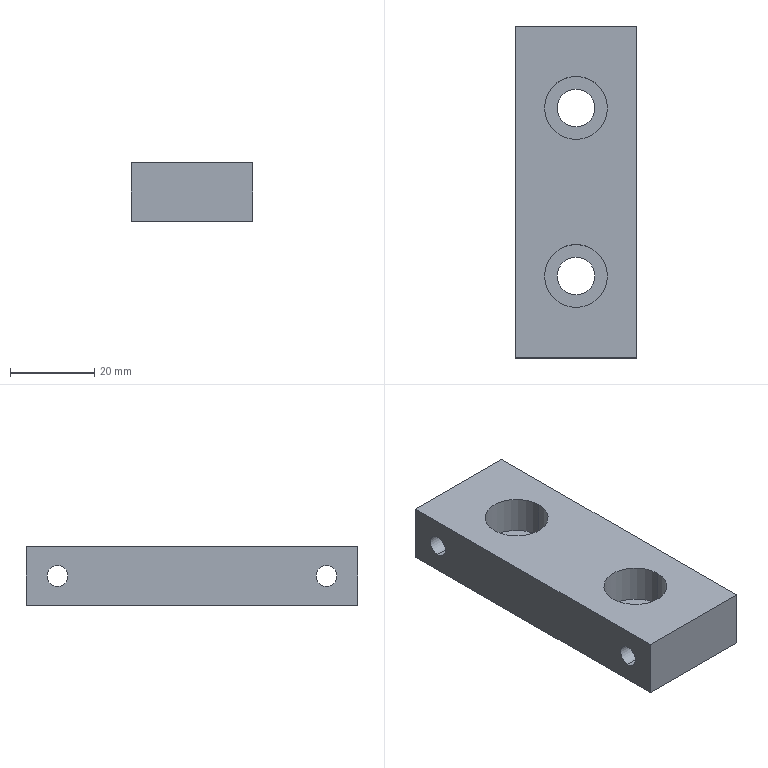Part | STEP file | PN_0053 (reinforcing block) | 1 solid | 20 faces | box 29 x 79 x 14 mm | volume 27118 mm3 | cylinder 12 | plane 8 | commonest cylinder face diameters 5 x4 9 x4 15 x4
STEP:
#1=CARTESIAN_POINT('',(0.,0.,0.));
#2=DIRECTION('',(0.,0.,1.));
#3=DIRECTION('',(1.,0.,0.));
#4=AXIS2_PLACEMENT_3D('',#1,#2,#3);
#5=CARTESIAN_POINT('',(-14.5,32.,4.5));
#6=VERTEX_POINT('',#5);
#7=CARTESIAN_POINT('',(14.5,32.,4.5));
#8=VERTEX_POINT('',#7);
#9=CARTESIAN_POINT('',(14.5,32.,4.5));
#10=DIRECTION('',(1.,0.,0.));
#11=VECTOR('',#10,1.);
#12=LINE('',#9,#11);
#13=CARTESIAN_POINT('',(14.5,32.,7.));
#14=DIRECTION('',(1.,0.,0.));
#15=DIRECTION('',(0.,0.,-1.));
#16=AXIS2_PLACEMENT_3D('',#13,#14,#15);
#17=CYLINDRICAL_SURFACE('',#16,2.5);
#18=CARTESIAN_POINT('',(6.283,0.));
#19=DIRECTION('',(0.,1.));
#20=VECTOR('',#19,1.);
#21=LINE('',#18,#20);
#22=(GEOMETRIC_REPRESENTATION_CONTEXT(2)PARAMETRIC_REPRESENTATION_CONTEXT()REPRESENTATION_CONTEXT('',''));
#23=DEFINITIONAL_REPRESENTATION('',(#21),#22);
#24=PCURVE('',#17,#23);
#25=CARTESIAN_POINT('',(14.5,32.,7.));
#26=DIRECTION('',(1.,0.,0.));
#27=DIRECTION('',(0.,0.,-1.));
#28=AXIS2_PLACEMENT_3D('',#25,#26,#27);
#29=CYLINDRICAL_SURFACE('',#28,2.5);
#30=CARTESIAN_POINT('',(0.,0.));
#31=DIRECTION('',(0.,1.));
#32=VECTOR('',#31,1.);
#33=LINE('',#30,#32);
#34=(GEOMETRIC_REPRESENTATION_CONTEXT(2)PARAMETRIC_REPRESENTATION_CONTEXT()REPRESENTATION_CONTEXT('',''));
#35=DEFINITIONAL_REPRESENTATION('',(#33),#34);
#36=PCURVE('',#29,#35);
#37=SURFACE_CURVE('',#12,(#24,#36),.PCURVE_S1.);
#38=EDGE_CURVE('',#6,#8,#37,.T.);
#39=ORIENTED_EDGE('',*,*,#38,.T.);
#40=CARTESIAN_POINT('',(14.5,32.,9.5));
#41=VERTEX_POINT('',#40);
#42=CARTESIAN_POINT('',(14.5,32.,7.));
#43=DIRECTION('',(1.,0.,0.));
#44=DIRECTION('',(0.,0.,-1.));
#45=AXIS2_PLACEMENT_3D('',#42,#43,#44);
#46=CIRCLE('',#45,2.5);
#47=CARTESIAN_POINT('',(0.,0.));
#48=DIRECTION('',(1.,0.));
#49=VECTOR('',#48,1.);
#50=LINE('',#47,#49);
#51=(GEOMETRIC_REPRESENTATION_CONTEXT(2)PARAMETRIC_REPRESENTATION_CONTEXT()REPRESENTATION_CONTEXT('',''));
#52=DEFINITIONAL_REPRESENTATION('',(#50),#51);
#53=PCURVE('',#17,#52);
#54=CARTESIAN_POINT('',(14.5,-39.5,14.));
#55=DIRECTION('',(-1.,0.,0.));
#56=DIRECTION('',(0.,0.,1.));
#57=AXIS2_PLACEMENT_3D('',#54,#55,#56);
#58=PLANE('',#57);
#59=CARTESIAN_POINT('',(-9.5,71.5));
#60=CARTESIAN_POINT('',(-9.5,75.83));
#61=CARTESIAN_POINT('',(-5.75,73.665));
#62=CARTESIAN_POINT('',(-2.,71.5));
#63=CARTESIAN_POINT('',(-5.75,69.335));
#64=CARTESIAN_POINT('',(-9.5,67.17));
#65=CARTESIAN_POINT('',(-9.5,71.5));
#66=(BOUNDED_CURVE()B_SPLINE_CURVE(2,(#59,#60,#61,#62,#63,#64,#65),.UNSPECIFIED.,.T.,.F.)B_SPLINE_CURVE_WITH_KNOTS((1,2,2,2,2,1),(-2.094,0.,2.094,4.189,6.283,8.378),.UNSPECIFIED.)CURVE()GEOMETRIC_REPRESENTATION_ITEM()RATIONAL_B_SPLINE_CURVE((1.,0.5,1.,0.5,1.,0.5,1.))REPRESENTATION_ITEM(''));
#67=(GEOMETRIC_REPRESENTATION_CONTEXT(2)PARAMETRIC_REPRESENTATION_CONTEXT()REPRESENTATION_CONTEXT('',''));
#68=DEFINITIONAL_REPRESENTATION('',(#66),#67);
#69=PCURVE('',#58,#68);
#70=SURFACE_CURVE('',#46,(#53,#69),.PCURVE_S1.);
#71=EDGE_CURVE('',#41,#8,#70,.T.);
#72=ORIENTED_EDGE('',*,*,#71,.F.);
#73=CARTESIAN_POINT('',(-14.5,32.,9.5));
#74=VERTEX_POINT('',#73);
#75=CARTESIAN_POINT('',(14.5,32.,9.5));
#76=DIRECTION('',(1.,0.,0.));
#77=VECTOR('',#76,1.);
#78=LINE('',#75,#77);
#79=CARTESIAN_POINT('',(3.142,0.));
#80=DIRECTION('',(0.,1.));
#81=VECTOR('',#80,1.);
#82=LINE('',#79,#81);
#83=(GEOMETRIC_REPRESENTATION_CONTEXT(2)PARAMETRIC_REPRESENTATION_CONTEXT()REPRESENTATION_CONTEXT('',''));
#84=DEFINITIONAL_REPRESENTATION('',(#82),#83);
#85=PCURVE('',#17,#84);
#86=CARTESIAN_POINT('',(3.142,0.));
#87=DIRECTION('',(0.,1.));
#88=VECTOR('',#87,1.);
#89=LINE('',#86,#88);
#90=(GEOMETRIC_REPRESENTATION_CONTEXT(2)PARAMETRIC_REPRESENTATION_CONTEXT()REPRESENTATION_CONTEXT('',''));
#91=DEFINITIONAL_REPRESENTATION('',(#89),#90);
#92=PCURVE('',#29,#91);
#93=SURFACE_CURVE('',#78,(#85,#92),.PCURVE_S1.);
#94=EDGE_CURVE('',#74,#41,#93,.T.);
#95=ORIENTED_EDGE('',*,*,#94,.F.);
#96=CARTESIAN_POINT('',(-14.5,32.,7.));
#97=DIRECTION('',(1.,0.,0.));
#98=DIRECTION('',(0.,0.,-1.));
#99=AXIS2_PLACEMENT_3D('',#96,#97,#98);
#100=CIRCLE('',#99,2.5);
#101=CARTESIAN_POINT('',(0.,-29.));
#102=DIRECTION('',(1.,0.));
#103=VECTOR('',#102,1.);
#104=LINE('',#101,#103);
#105=(GEOMETRIC_REPRESENTATION_CONTEXT(2)PARAMETRIC_REPRESENTATION_CONTEXT()REPRESENTATION_CONTEXT('',''));
#106=DEFINITIONAL_REPRESENTATION('',(#104),#105);
#107=PCURVE('',#17,#106);
#108=CARTESIAN_POINT('',(-14.5,-39.5,14.));
#109=DIRECTION('',(1.,0.,0.));
#110=DIRECTION('',(0.,0.,-1.));
#111=AXIS2_PLACEMENT_3D('',#108,#109,#110);
#112=PLANE('',#111);
#113=CARTESIAN_POINT('',(7.,71.5));
#114=DIRECTION('',(1.,0.));
#115=AXIS2_PLACEMENT_2D('',#113,#114);
#116=CIRCLE('',#115,2.5);
#117=(GEOMETRIC_REPRESENTATION_CONTEXT(2)PARAMETRIC_REPRESENTATION_CONTEXT()REPRESENTATION_CONTEXT('',''));
#118=DEFINITIONAL_REPRESENTATION('',(#116),#117);
#119=PCURVE('',#112,#118);
#120=SURFACE_CURVE('',#100,(#107,#119),.PCURVE_S1.);
#121=EDGE_CURVE('',#74,#6,#120,.T.);
#122=ORIENTED_EDGE('',*,*,#121,.T.);
#123=EDGE_LOOP('',(#39,#72,#95,#122));
#124=FACE_BOUND('',#123,.F.);
#125=ADVANCED_FACE('',(#124),#17,.F.);
#126=CARTESIAN_POINT('',(-14.5,-32.,4.5));
#127=VERTEX_POINT('',#126);
#128=CARTESIAN_POINT('',(14.5,-32.,4.5));
#129=VERTEX_POINT('',#128);
#130=CARTESIAN_POINT('',(14.5,-32.,4.5));
#131=DIRECTION('',(1.,0.,0.));
#132=VECTOR('',#131,1.);
#133=LINE('',#130,#132);
#134=CARTESIAN_POINT('',(14.5,-32.,7.));
#135=DIRECTION('',(1.,0.,0.));
#136=DIRECTION('',(0.,0.,-1.));
#137=AXIS2_PLACEMENT_3D('',#134,#135,#136);
#138=CYLINDRICAL_SURFACE('',#137,2.5);
#139=CARTESIAN_POINT('',(6.283,0.));
#140=DIRECTION('',(0.,1.));
#141=VECTOR('',#140,1.);
#142=LINE('',#139,#141);
#143=(GEOMETRIC_REPRESENTATION_CONTEXT(2)PARAMETRIC_REPRESENTATION_CONTEXT()REPRESENTATION_CONTEXT('',''));
#144=DEFINITIONAL_REPRESENTATION('',(#142),#143);
#145=PCURVE('',#138,#144);
#146=CARTESIAN_POINT('',(14.5,-32.,7.));
#147=DIRECTION('',(1.,0.,0.));
#148=DIRECTION('',(0.,0.,-1.));
#149=AXIS2_PLACEMENT_3D('',#146,#147,#148);
#150=CYLINDRICAL_SURFACE('',#149,2.5);
#151=CARTESIAN_POINT('',(0.,0.));
#152=DIRECTION('',(0.,1.));
#153=VECTOR('',#152,1.);
#154=LINE('',#151,#153);
#155=(GEOMETRIC_REPRESENTATION_CONTEXT(2)PARAMETRIC_REPRESENTATION_CONTEXT()REPRESENTATION_CONTEXT('',''));
#156=DEFINITIONAL_REPRESENTATION('',(#154),#155);
#157=PCURVE('',#150,#156);
#158=SURFACE_CURVE('',#133,(#145,#157),.PCURVE_S1.);
#159=EDGE_CURVE('',#127,#129,#158,.T.);
#160=ORIENTED_EDGE('',*,*,#159,.T.);
#161=CARTESIAN_POINT('',(14.5,-32.,9.5));
#162=VERTEX_POINT('',#161);
#163=CARTESIAN_POINT('',(14.5,-32.,7.));
#164=DIRECTION('',(1.,0.,0.));
#165=DIRECTION('',(0.,0.,-1.));
#166=AXIS2_PLACEMENT_3D('',#163,#164,#165);
#167=CIRCLE('',#166,2.5);
#168=CARTESIAN_POINT('',(0.,0.));
#169=DIRECTION('',(1.,0.));
#170=VECTOR('',#169,1.);
#171=LINE('',#168,#170);
#172=(GEOMETRIC_REPRESENTATION_CONTEXT(2)PARAMETRIC_REPRESENTATION_CONTEXT()REPRESENTATION_CONTEXT('',''));
#173=DEFINITIONAL_REPRESENTATION('',(#171),#172);
#174=PCURVE('',#138,#173);
#175=CARTESIAN_POINT('',(-9.5,7.5));
#176=CARTESIAN_POINT('',(-9.5,11.83));
#177=CARTESIAN_POINT('',(-5.75,9.665));
#178=CARTESIAN_POINT('',(-2.,7.5));
#179=CARTESIAN_POINT('',(-5.75,5.335));
#180=CARTESIAN_POINT('',(-9.5,3.17));
#181=CARTESIAN_POINT('',(-9.5,7.5));
#182=(BOUNDED_CURVE()B_SPLINE_CURVE(2,(#175,#176,#177,#178,#179,#180,#181),.UNSPECIFIED.,.T.,.F.)B_SPLINE_CURVE_WITH_KNOTS((1,2,2,2,2,1),(-2.094,0.,2.094,4.189,6.283,8.378),.UNSPECIFIED.)CURVE()GEOMETRIC_REPRESENTATION_ITEM()RATIONAL_B_SPLINE_CURVE((1.,0.5,1.,0.5,1.,0.5,1.))REPRESENTATION_ITEM(''));
#183=(GEOMETRIC_REPRESENTATION_CONTEXT(2)PARAMETRIC_REPRESENTATION_CONTEXT()REPRESENTATION_CONTEXT('',''));
#184=DEFINITIONAL_REPRESENTATION('',(#182),#183);
#185=PCURVE('',#58,#184);
#186=SURFACE_CURVE('',#167,(#174,#185),.PCURVE_S1.);
#187=EDGE_CURVE('',#162,#129,#186,.T.);
#188=ORIENTED_EDGE('',*,*,#187,.F.);
#189=CARTESIAN_POINT('',(-14.5,-32.,9.5));
#190=VERTEX_POINT('',#189);
#191=CARTESIAN_POINT('',(14.5,-32.,9.5));
#192=DIRECTION('',(1.,0.,0.));
#193=VECTOR('',#192,1.);
#194=LINE('',#191,#193);
#195=CARTESIAN_POINT('',(3.142,0.));
#196=DIRECTION('',(0.,1.));
#197=VECTOR('',#196,1.);
#198=LINE('',#195,#197);
#199=(GEOMETRIC_REPRESENTATION_CONTEXT(2)PARAMETRIC_REPRESENTATION_CONTEXT()REPRESENTATION_CONTEXT('',''));
#200=DEFINITIONAL_REPRESENTATION('',(#198),#199);
#201=PCURVE('',#138,#200);
#202=CARTESIAN_POINT('',(3.142,0.));
#203=DIRECTION('',(0.,1.));
#204=VECTOR('',#203,1.);
#205=LINE('',#202,#204);
#206=(GEOMETRIC_REPRESENTATION_CONTEXT(2)PARAMETRIC_REPRESENTATION_CONTEXT()REPRESENTATION_CONTEXT('',''));
#207=DEFINITIONAL_REPRESENTATION('',(#205),#206);
#208=PCURVE('',#150,#207);
#209=SURFACE_CURVE('',#194,(#201,#208),.PCURVE_S1.);
#210=EDGE_CURVE('',#190,#162,#209,.T.);
#211=ORIENTED_EDGE('',*,*,#210,.F.);
#212=CARTESIAN_POINT('',(-14.5,-32.,7.));
#213=DIRECTION('',(1.,0.,0.));
#214=DIRECTION('',(0.,0.,-1.));
#215=AXIS2_PLACEMENT_3D('',#212,#213,#214);
#216=CIRCLE('',#215,2.5);
#217=CARTESIAN_POINT('',(0.,-29.));
#218=DIRECTION('',(1.,0.));
#219=VECTOR('',#218,1.);
#220=LINE('',#217,#219);
#221=(GEOMETRIC_REPRESENTATION_CONTEXT(2)PARAMETRIC_REPRESENTATION_CONTEXT()REPRESENTATION_CONTEXT('',''));
#222=DEFINITIONAL_REPRESENTATION('',(#220),#221);
#223=PCURVE('',#138,#222);
#224=CARTESIAN_POINT('',(7.,7.5));
#225=DIRECTION('',(1.,0.));
#226=AXIS2_PLACEMENT_2D('',#224,#225);
#227=CIRCLE('',#226,2.5);
#228=(GEOMETRIC_REPRESENTATION_CONTEXT(2)PARAMETRIC_REPRESENTATION_CONTEXT()REPRESENTATION_CONTEXT('',''));
#229=DEFINITIONAL_REPRESENTATION('',(#227),#228);
#230=PCURVE('',#112,#229);
#231=SURFACE_CURVE('',#216,(#223,#230),.PCURVE_S1.);
#232=EDGE_CURVE('',#190,#127,#231,.T.);
#233=ORIENTED_EDGE('',*,*,#232,.T.);
#234=EDGE_LOOP('',(#160,#188,#211,#233));
#235=FACE_BOUND('',#234,.F.);
#236=ADVANCED_FACE('',(#235),#138,.F.);
#237=CARTESIAN_POINT('',(7.5,20.,5.));
#238=VERTEX_POINT('',#237);
#239=CARTESIAN_POINT('',(7.5,20.,14.));
#240=VERTEX_POINT('',#239);
#241=CARTESIAN_POINT('',(7.5,20.,14.));
#242=DIRECTION('',(0.,0.,1.));
#243=VECTOR('',#242,1.);
#244=LINE('',#241,#243);
#245=CARTESIAN_POINT('',(0.,20.,14.));
#246=DIRECTION('',(0.,0.,1.));
#247=DIRECTION('',(1.,0.,0.));
#248=AXIS2_PLACEMENT_3D('',#245,#246,#247);
#249=CYLINDRICAL_SURFACE('',#248,7.5);
#250=CARTESIAN_POINT('',(6.283,0.));
#251=DIRECTION('',(0.,1.));
#252=VECTOR('',#251,1.);
#253=LINE('',#250,#252);
#254=(GEOMETRIC_REPRESENTATION_CONTEXT(2)PARAMETRIC_REPRESENTATION_CONTEXT()REPRESENTATION_CONTEXT('',''));
#255=DEFINITIONAL_REPRESENTATION('',(#253),#254);
#256=PCURVE('',#249,#255);
#257=CARTESIAN_POINT('',(0.,20.,14.));
#258=DIRECTION('',(0.,0.,1.));
#259=DIRECTION('',(1.,0.,0.));
#260=AXIS2_PLACEMENT_3D('',#257,#258,#259);
#261=CYLINDRICAL_SURFACE('',#260,7.5);
#262=CARTESIAN_POINT('',(0.,0.));
#263=DIRECTION('',(0.,1.));
#264=VECTOR('',#263,1.);
#265=LINE('',#262,#264);
#266=(GEOMETRIC_REPRESENTATION_CONTEXT(2)PARAMETRIC_REPRESENTATION_CONTEXT()REPRESENTATION_CONTEXT('',''));
#267=DEFINITIONAL_REPRESENTATION('',(#265),#266);
#268=PCURVE('',#261,#267);
#269=SURFACE_CURVE('',#244,(#256,#268),.PCURVE_S1.);
#270=EDGE_CURVE('',#238,#240,#269,.T.);
#271=ORIENTED_EDGE('',*,*,#270,.T.);
#272=CARTESIAN_POINT('',(-7.5,20.,14.));
#273=VERTEX_POINT('',#272);
#274=CARTESIAN_POINT('',(0.,20.,14.));
#275=DIRECTION('',(0.,0.,1.));
#276=DIRECTION('',(1.,0.,0.));
#277=AXIS2_PLACEMENT_3D('',#274,#275,#276);
#278=CIRCLE('',#277,7.5);
#279=CARTESIAN_POINT('',(0.,0.));
#280=DIRECTION('',(1.,0.));
#281=VECTOR('',#280,1.);
#282=LINE('',#279,#281);
#283=(GEOMETRIC_REPRESENTATION_CONTEXT(2)PARAMETRIC_REPRESENTATION_CONTEXT()REPRESENTATION_CONTEXT('',''));
#284=DEFINITIONAL_REPRESENTATION('',(#282),#283);
#285=PCURVE('',#249,#284);
#286=CARTESIAN_POINT('',(0.,0.,14.));
#287=DIRECTION('',(0.,0.,1.));
#288=DIRECTION('',(1.,0.,0.));
#289=AXIS2_PLACEMENT_3D('',#286,#287,#288);
#290=PLANE('',#289);
#291=CARTESIAN_POINT('',(0.,20.));
#292=DIRECTION('',(1.,0.));
#293=AXIS2_PLACEMENT_2D('',#291,#292);
#294=CIRCLE('',#293,7.5);
#295=(GEOMETRIC_REPRESENTATION_CONTEXT(2)PARAMETRIC_REPRESENTATION_CONTEXT()REPRESENTATION_CONTEXT('',''));
#296=DEFINITIONAL_REPRESENTATION('',(#294),#295);
#297=PCURVE('',#290,#296);
#298=SURFACE_CURVE('',#278,(#285,#297),.PCURVE_S1.);
#299=EDGE_CURVE('',#273,#240,#298,.T.);
#300=ORIENTED_EDGE('',*,*,#299,.F.);
#301=CARTESIAN_POINT('',(-7.5,20.,5.));
#302=VERTEX_POINT('',#301);
#303=CARTESIAN_POINT('',(-7.5,20.,14.));
#304=DIRECTION('',(0.,0.,1.));
#305=VECTOR('',#304,1.);
#306=LINE('',#303,#305);
#307=CARTESIAN_POINT('',(3.142,0.));
#308=DIRECTION('',(0.,1.));
#309=VECTOR('',#308,1.);
#310=LINE('',#307,#309);
#311=(GEOMETRIC_REPRESENTATION_CONTEXT(2)PARAMETRIC_REPRESENTATION_CONTEXT()REPRESENTATION_CONTEXT('',''));
#312=DEFINITIONAL_REPRESENTATION('',(#310),#311);
#313=PCURVE('',#249,#312);
#314=CARTESIAN_POINT('',(3.142,0.));
#315=DIRECTION('',(0.,1.));
#316=VECTOR('',#315,1.);
#317=LINE('',#314,#316);
#318=(GEOMETRIC_REPRESENTATION_CONTEXT(2)PARAMETRIC_REPRESENTATION_CONTEXT()REPRESENTATION_CONTEXT('',''));
#319=DEFINITIONAL_REPRESENTATION('',(#317),#318);
#320=PCURVE('',#261,#319);
#321=SURFACE_CURVE('',#306,(#313,#320),.PCURVE_S1.);
#322=EDGE_CURVE('',#302,#273,#321,.T.);
#323=ORIENTED_EDGE('',*,*,#322,.F.);
#324=CARTESIAN_POINT('',(0.,20.,5.));
#325=DIRECTION('',(0.,0.,1.));
#326=DIRECTION('',(1.,0.,0.));
#327=AXIS2_PLACEMENT_3D('',#324,#325,#326);
#328=CIRCLE('',#327,7.5);
#329=CARTESIAN_POINT('',(0.,-9.));
#330=DIRECTION('',(1.,0.));
#331=VECTOR('',#330,1.);
#332=LINE('',#329,#331);
#333=(GEOMETRIC_REPRESENTATION_CONTEXT(2)PARAMETRIC_REPRESENTATION_CONTEXT()REPRESENTATION_CONTEXT('',''));
#334=DEFINITIONAL_REPRESENTATION('',(#332),#333);
#335=PCURVE('',#249,#334);
#336=CARTESIAN_POINT('',(4.5,20.,5.));
#337=DIRECTION('',(0.,0.,-1.));
#338=DIRECTION('',(-1.,0.,0.));
#339=AXIS2_PLACEMENT_3D('',#336,#337,#338);
#340=PLANE('',#339);
#341=CARTESIAN_POINT('',(-3.,0.));
#342=CARTESIAN_POINT('',(-3.,12.99));
#343=CARTESIAN_POINT('',(8.25,6.495));
#344=CARTESIAN_POINT('',(19.5,0.));
#345=CARTESIAN_POINT('',(8.25,-6.495));
#346=CARTESIAN_POINT('',(-3.,-12.99));
#347=CARTESIAN_POINT('',(-3.,0.));
#348=(BOUNDED_CURVE()B_SPLINE_CURVE(2,(#341,#342,#343,#344,#345,#346,#347),.UNSPECIFIED.,.T.,.F.)B_SPLINE_CURVE_WITH_KNOTS((1,2,2,2,2,1),(-2.094,0.,2.094,4.189,6.283,8.378),.UNSPECIFIED.)CURVE()GEOMETRIC_REPRESENTATION_ITEM()RATIONAL_B_SPLINE_CURVE((1.,0.5,1.,0.5,1.,0.5,1.))REPRESENTATION_ITEM(''));
#349=(GEOMETRIC_REPRESENTATION_CONTEXT(2)PARAMETRIC_REPRESENTATION_CONTEXT()REPRESENTATION_CONTEXT('',''));
#350=DEFINITIONAL_REPRESENTATION('',(#348),#349);
#351=PCURVE('',#340,#350);
#352=SURFACE_CURVE('',#328,(#335,#351),.PCURVE_S1.);
#353=EDGE_CURVE('',#302,#238,#352,.T.);
#354=ORIENTED_EDGE('',*,*,#353,.T.);
#355=EDGE_LOOP('',(#271,#300,#323,#354));
#356=FACE_BOUND('',#355,.F.);
#357=ADVANCED_FACE('',(#356),#249,.F.);
#358=CARTESIAN_POINT('',(4.5,20.,0.));
#359=VERTEX_POINT('',#358);
#360=CARTESIAN_POINT('',(4.5,20.,5.));
#361=VERTEX_POINT('',#360);
#362=CARTESIAN_POINT('',(4.5,20.,14.));
#363=DIRECTION('',(0.,0.,1.));
#364=VECTOR('',#363,1.);
#365=LINE('',#362,#364);
#366=CARTESIAN_POINT('',(0.,20.,14.));
#367=DIRECTION('',(0.,0.,1.));
#368=DIRECTION('',(1.,0.,0.));
#369=AXIS2_PLACEMENT_3D('',#366,#367,#368);
#370=CYLINDRICAL_SURFACE('',#369,4.5);
#371=CARTESIAN_POINT('',(6.283,0.));
#372=DIRECTION('',(0.,1.));
#373=VECTOR('',#372,1.);
#374=LINE('',#371,#373);
#375=(GEOMETRIC_REPRESENTATION_CONTEXT(2)PARAMETRIC_REPRESENTATION_CONTEXT()REPRESENTATION_CONTEXT('',''));
#376=DEFINITIONAL_REPRESENTATION('',(#374),#375);
#377=PCURVE('',#370,#376);
#378=CARTESIAN_POINT('',(0.,20.,14.));
#379=DIRECTION('',(0.,0.,1.));
#380=DIRECTION('',(1.,0.,0.));
#381=AXIS2_PLACEMENT_3D('',#378,#379,#380);
#382=CYLINDRICAL_SURFACE('',#381,4.5);
#383=CARTESIAN_POINT('',(0.,0.));
#384=DIRECTION('',(0.,1.));
#385=VECTOR('',#384,1.);
#386=LINE('',#383,#385);
#387=(GEOMETRIC_REPRESENTATION_CONTEXT(2)PARAMETRIC_REPRESENTATION_CONTEXT()REPRESENTATION_CONTEXT('',''));
#388=DEFINITIONAL_REPRESENTATION('',(#386),#387);
#389=PCURVE('',#382,#388);
#390=SURFACE_CURVE('',#365,(#377,#389),.PCURVE_S1.);
#391=EDGE_CURVE('',#359,#361,#390,.T.);
#392=ORIENTED_EDGE('',*,*,#391,.T.);
#393=CARTESIAN_POINT('',(-4.5,20.,5.));
#394=VERTEX_POINT('',#393);
#395=CARTESIAN_POINT('',(0.,20.,5.));
#396=DIRECTION('',(0.,0.,1.));
#397=DIRECTION('',(1.,0.,0.));
#398=AXIS2_PLACEMENT_3D('',#395,#396,#397);
#399=CIRCLE('',#398,4.5);
#400=CARTESIAN_POINT('',(0.,-9.));
#401=DIRECTION('',(1.,0.));
#402=VECTOR('',#401,1.);
#403=LINE('',#400,#402);
#404=(GEOMETRIC_REPRESENTATION_CONTEXT(2)PARAMETRIC_REPRESENTATION_CONTEXT()REPRESENTATION_CONTEXT('',''));
#405=DEFINITIONAL_REPRESENTATION('',(#403),#404);
#406=PCURVE('',#370,#405);
#407=CARTESIAN_POINT('',(0.,0.));
#408=CARTESIAN_POINT('',(0.,7.794));
#409=CARTESIAN_POINT('',(6.75,3.897));
#410=CARTESIAN_POINT('',(13.5,0.));
#411=CARTESIAN_POINT('',(6.75,-3.897));
#412=CARTESIAN_POINT('',(0.,-7.794));
#413=CARTESIAN_POINT('',(0.,0.));
#414=(BOUNDED_CURVE()B_SPLINE_CURVE(2,(#407,#408,#409,#410,#411,#412,#413),.UNSPECIFIED.,.T.,.F.)B_SPLINE_CURVE_WITH_KNOTS((1,2,2,2,2,1),(-2.094,0.,2.094,4.189,6.283,8.378),.UNSPECIFIED.)CURVE()GEOMETRIC_REPRESENTATION_ITEM()RATIONAL_B_SPLINE_CURVE((1.,0.5,1.,0.5,1.,0.5,1.))REPRESENTATION_ITEM(''));
#415=(GEOMETRIC_REPRESENTATION_CONTEXT(2)PARAMETRIC_REPRESENTATION_CONTEXT()REPRESENTATION_CONTEXT('',''));
#416=DEFINITIONAL_REPRESENTATION('',(#414),#415);
#417=PCURVE('',#340,#416);
#418=SURFACE_CURVE('',#399,(#406,#417),.PCURVE_S1.);
#419=EDGE_CURVE('',#394,#361,#418,.T.);
#420=ORIENTED_EDGE('',*,*,#419,.F.);
#421=CARTESIAN_POINT('',(-4.5,20.,0.));
#422=VERTEX_POINT('',#421);
#423=CARTESIAN_POINT('',(-4.5,20.,14.));
#424=DIRECTION('',(0.,0.,1.));
#425=VECTOR('',#424,1.);
#426=LINE('',#423,#425);
#427=CARTESIAN_POINT('',(3.142,0.));
#428=DIRECTION('',(0.,1.));
#429=VECTOR('',#428,1.);
#430=LINE('',#427,#429);
#431=(GEOMETRIC_REPRESENTATION_CONTEXT(2)PARAMETRIC_REPRESENTATION_CONTEXT()REPRESENTATION_CONTEXT('',''));
#432=DEFINITIONAL_REPRESENTATION('',(#430),#431);
#433=PCURVE('',#370,#432);
#434=CARTESIAN_POINT('',(3.142,0.));
#435=DIRECTION('',(0.,1.));
#436=VECTOR('',#435,1.);
#437=LINE('',#434,#436);
#438=(GEOMETRIC_REPRESENTATION_CONTEXT(2)PARAMETRIC_REPRESENTATION_CONTEXT()REPRESENTATION_CONTEXT('',''));
#439=DEFINITIONAL_REPRESENTATION('',(#437),#438);
#440=PCURVE('',#382,#439);
#441=SURFACE_CURVE('',#426,(#433,#440),.PCURVE_S1.);
#442=EDGE_CURVE('',#422,#394,#441,.T.);
#443=ORIENTED_EDGE('',*,*,#442,.F.);
#444=CARTESIAN_POINT('',(0.,20.,0.));
#445=DIRECTION('',(0.,0.,1.));
#446=DIRECTION('',(1.,0.,0.));
#447=AXIS2_PLACEMENT_3D('',#444,#445,#446);
#448=CIRCLE('',#447,4.5);
#449=CARTESIAN_POINT('',(0.,-14.));
#450=DIRECTION('',(1.,0.));
#451=VECTOR('',#450,1.);
#452=LINE('',#449,#451);
#453=(GEOMETRIC_REPRESENTATION_CONTEXT(2)PARAMETRIC_REPRESENTATION_CONTEXT()REPRESENTATION_CONTEXT('',''));
#454=DEFINITIONAL_REPRESENTATION('',(#452),#453);
#455=PCURVE('',#370,#454);
#456=CARTESIAN_POINT('',(0.,0.,0.));
#457=DIRECTION('',(0.,0.,1.));
#458=DIRECTION('',(1.,0.,0.));
#459=AXIS2_PLACEMENT_3D('',#456,#457,#458);
#460=PLANE('',#459);
#461=CARTESIAN_POINT('',(0.,20.));
#462=DIRECTION('',(1.,0.));
#463=AXIS2_PLACEMENT_2D('',#461,#462);
#464=CIRCLE('',#463,4.5);
#465=(GEOMETRIC_REPRESENTATION_CONTEXT(2)PARAMETRIC_REPRESENTATION_CONTEXT()REPRESENTATION_CONTEXT('',''));
#466=DEFINITIONAL_REPRESENTATION('',(#464),#465);
#467=PCURVE('',#460,#466);
#468=SURFACE_CURVE('',#448,(#455,#467),.PCURVE_S1.);
#469=EDGE_CURVE('',#422,#359,#468,.T.);
#470=ORIENTED_EDGE('',*,*,#469,.T.);
#471=EDGE_LOOP('',(#392,#420,#443,#470));
#472=FACE_BOUND('',#471,.F.);
#473=ADVANCED_FACE('',(#472),#370,.F.);
#474=CARTESIAN_POINT('',(7.5,-20.,5.));
#475=VERTEX_POINT('',#474);
#476=CARTESIAN_POINT('',(7.5,-20.,14.));
#477=VERTEX_POINT('',#476);
#478=CARTESIAN_POINT('',(7.5,-20.,14.));
#479=DIRECTION('',(0.,0.,1.));
#480=VECTOR('',#479,1.);
#481=LINE('',#478,#480);
#482=CARTESIAN_POINT('',(0.,-20.,14.));
#483=DIRECTION('',(0.,0.,1.));
#484=DIRECTION('',(1.,0.,0.));
#485=AXIS2_PLACEMENT_3D('',#482,#483,#484);
#486=CYLINDRICAL_SURFACE('',#485,7.5);
#487=CARTESIAN_POINT('',(6.283,0.));
#488=DIRECTION('',(0.,1.));
#489=VECTOR('',#488,1.);
#490=LINE('',#487,#489);
#491=(GEOMETRIC_REPRESENTATION_CONTEXT(2)PARAMETRIC_REPRESENTATION_CONTEXT()REPRESENTATION_CONTEXT('',''));
#492=DEFINITIONAL_REPRESENTATION('',(#490),#491);
#493=PCURVE('',#486,#492);
#494=CARTESIAN_POINT('',(0.,-20.,14.));
#495=DIRECTION('',(0.,0.,1.));
#496=DIRECTION('',(1.,0.,0.));
#497=AXIS2_PLACEMENT_3D('',#494,#495,#496);
#498=CYLINDRICAL_SURFACE('',#497,7.5);
#499=CARTESIAN_POINT('',(0.,0.));
#500=DIRECTION('',(0.,1.));
#501=VECTOR('',#500,1.);
#502=LINE('',#499,#501);
#503=(GEOMETRIC_REPRESENTATION_CONTEXT(2)PARAMETRIC_REPRESENTATION_CONTEXT()REPRESENTATION_CONTEXT('',''));
#504=DEFINITIONAL_REPRESENTATION('',(#502),#503);
#505=PCURVE('',#498,#504);
#506=SURFACE_CURVE('',#481,(#493,#505),.PCURVE_S1.);
#507=EDGE_CURVE('',#475,#477,#506,.T.);
#508=ORIENTED_EDGE('',*,*,#507,.T.);
#509=CARTESIAN_POINT('',(-7.5,-20.,14.));
#510=VERTEX_POINT('',#509);
#511=CARTESIAN_POINT('',(0.,-20.,14.));
#512=DIRECTION('',(0.,0.,1.));
#513=DIRECTION('',(1.,0.,0.));
#514=AXIS2_PLACEMENT_3D('',#511,#512,#513);
#515=CIRCLE('',#514,7.5);
#516=CARTESIAN_POINT('',(0.,0.));
#517=DIRECTION('',(1.,0.));
#518=VECTOR('',#517,1.);
#519=LINE('',#516,#518);
#520=(GEOMETRIC_REPRESENTATION_CONTEXT(2)PARAMETRIC_REPRESENTATION_CONTEXT()REPRESENTATION_CONTEXT('',''));
#521=DEFINITIONAL_REPRESENTATION('',(#519),#520);
#522=PCURVE('',#486,#521);
#523=CARTESIAN_POINT('',(0.,-20.));
#524=DIRECTION('',(1.,0.));
#525=AXIS2_PLACEMENT_2D('',#523,#524);
#526=CIRCLE('',#525,7.5);
#527=(GEOMETRIC_REPRESENTATION_CONTEXT(2)PARAMETRIC_REPRESENTATION_CONTEXT()REPRESENTATION_CONTEXT('',''));
#528=DEFINITIONAL_REPRESENTATION('',(#526),#527);
#529=PCURVE('',#290,#528);
#530=SURFACE_CURVE('',#515,(#522,#529),.PCURVE_S1.);
#531=EDGE_CURVE('',#510,#477,#530,.T.);
#532=ORIENTED_EDGE('',*,*,#531,.F.);
#533=CARTESIAN_POINT('',(-7.5,-20.,5.));
#534=VERTEX_POINT('',#533);
#535=CARTESIAN_POINT('',(-7.5,-20.,14.));
#536=DIRECTION('',(0.,0.,1.));
#537=VECTOR('',#536,1.);
#538=LINE('',#535,#537);
#539=CARTESIAN_POINT('',(3.142,0.));
#540=DIRECTION('',(0.,1.));
#541=VECTOR('',#540,1.);
#542=LINE('',#539,#541);
#543=(GEOMETRIC_REPRESENTATION_CONTEXT(2)PARAMETRIC_REPRESENTATION_CONTEXT()REPRESENTATION_CONTEXT('',''));
#544=DEFINITIONAL_REPRESENTATION('',(#542),#543);
#545=PCURVE('',#486,#544);
#546=CARTESIAN_POINT('',(3.142,0.));
#547=DIRECTION('',(0.,1.));
#548=VECTOR('',#547,1.);
#549=LINE('',#546,#548);
#550=(GEOMETRIC_REPRESENTATION_CONTEXT(2)PARAMETRIC_REPRESENTATION_CONTEXT()REPRESENTATION_CONTEXT('',''));
#551=DEFINITIONAL_REPRESENTATION('',(#549),#550);
#552=PCURVE('',#498,#551);
#553=SURFACE_CURVE('',#538,(#545,#552),.PCURVE_S1.);
#554=EDGE_CURVE('',#534,#510,#553,.T.);
#555=ORIENTED_EDGE('',*,*,#554,.F.);
#556=CARTESIAN_POINT('',(0.,-20.,5.));
#557=DIRECTION('',(0.,0.,1.));
#558=DIRECTION('',(1.,0.,0.));
#559=AXIS2_PLACEMENT_3D('',#556,#557,#558);
#560=CIRCLE('',#559,7.5);
#561=CARTESIAN_POINT('',(0.,-9.));
#562=DIRECTION('',(1.,0.));
#563=VECTOR('',#562,1.);
#564=LINE('',#561,#563);
#565=(GEOMETRIC_REPRESENTATION_CONTEXT(2)PARAMETRIC_REPRESENTATION_CONTEXT()REPRESENTATION_CONTEXT('',''));
#566=DEFINITIONAL_REPRESENTATION('',(#564),#565);
#567=PCURVE('',#486,#566);
#568=CARTESIAN_POINT('',(4.5,-20.,5.));
#569=DIRECTION('',(0.,0.,-1.));
#570=DIRECTION('',(-1.,0.,0.));
#571=AXIS2_PLACEMENT_3D('',#568,#569,#570);
#572=PLANE('',#571);
#573=CARTESIAN_POINT('',(-3.,0.));
#574=CARTESIAN_POINT('',(-3.,12.99));
#575=CARTESIAN_POINT('',(8.25,6.495));
#576=CARTESIAN_POINT('',(19.5,0.));
#577=CARTESIAN_POINT('',(8.25,-6.495));
#578=CARTESIAN_POINT('',(-3.,-12.99));
#579=CARTESIAN_POINT('',(-3.,0.));
#580=(BOUNDED_CURVE()B_SPLINE_CURVE(2,(#573,#574,#575,#576,#577,#578,#579),.UNSPECIFIED.,.T.,.F.)B_SPLINE_CURVE_WITH_KNOTS((1,2,2,2,2,1),(-2.094,0.,2.094,4.189,6.283,8.378),.UNSPECIFIED.)CURVE()GEOMETRIC_REPRESENTATION_ITEM()RATIONAL_B_SPLINE_CURVE((1.,0.5,1.,0.5,1.,0.5,1.))REPRESENTATION_ITEM(''));
#581=(GEOMETRIC_REPRESENTATION_CONTEXT(2)PARAMETRIC_REPRESENTATION_CONTEXT()REPRESENTATION_CONTEXT('',''));
#582=DEFINITIONAL_REPRESENTATION('',(#580),#581);
#583=PCURVE('',#572,#582);
#584=SURFACE_CURVE('',#560,(#567,#583),.PCURVE_S1.);
#585=EDGE_CURVE('',#534,#475,#584,.T.);
#586=ORIENTED_EDGE('',*,*,#585,.T.);
#587=EDGE_LOOP('',(#508,#532,#555,#586));
#588=FACE_BOUND('',#587,.F.);
#589=ADVANCED_FACE('',(#588),#486,.F.);
#590=CARTESIAN_POINT('',(4.5,-20.,0.));
#591=VERTEX_POINT('',#590);
#592=CARTESIAN_POINT('',(4.5,-20.,5.));
#593=VERTEX_POINT('',#592);
#594=CARTESIAN_POINT('',(4.5,-20.,14.));
#595=DIRECTION('',(0.,0.,1.));
#596=VECTOR('',#595,1.);
#597=LINE('',#594,#596);
#598=CARTESIAN_POINT('',(0.,-20.,14.));
#599=DIRECTION('',(0.,0.,1.));
#600=DIRECTION('',(1.,0.,0.));
#601=AXIS2_PLACEMENT_3D('',#598,#599,#600);
#602=CYLINDRICAL_SURFACE('',#601,4.5);
#603=CARTESIAN_POINT('',(6.283,0.));
#604=DIRECTION('',(0.,1.));
#605=VECTOR('',#604,1.);
#606=LINE('',#603,#605);
#607=(GEOMETRIC_REPRESENTATION_CONTEXT(2)PARAMETRIC_REPRESENTATION_CONTEXT()REPRESENTATION_CONTEXT('',''));
#608=DEFINITIONAL_REPRESENTATION('',(#606),#607);
#609=PCURVE('',#602,#608);
#610=CARTESIAN_POINT('',(0.,-20.,14.));
#611=DIRECTION('',(0.,0.,1.));
#612=DIRECTION('',(1.,0.,0.));
#613=AXIS2_PLACEMENT_3D('',#610,#611,#612);
#614=CYLINDRICAL_SURFACE('',#613,4.5);
#615=CARTESIAN_POINT('',(0.,0.));
#616=DIRECTION('',(0.,1.));
#617=VECTOR('',#616,1.);
#618=LINE('',#615,#617);
#619=(GEOMETRIC_REPRESENTATION_CONTEXT(2)PARAMETRIC_REPRESENTATION_CONTEXT()REPRESENTATION_CONTEXT('',''));
#620=DEFINITIONAL_REPRESENTATION('',(#618),#619);
#621=PCURVE('',#614,#620);
#622=SURFACE_CURVE('',#597,(#609,#621),.PCURVE_S1.);
#623=EDGE_CURVE('',#591,#593,#622,.T.);
#624=ORIENTED_EDGE('',*,*,#623,.T.);
#625=CARTESIAN_POINT('',(-4.5,-20.,5.));
#626=VERTEX_POINT('',#625);
#627=CARTESIAN_POINT('',(0.,-20.,5.));
#628=DIRECTION('',(0.,0.,1.));
#629=DIRECTION('',(1.,0.,0.));
#630=AXIS2_PLACEMENT_3D('',#627,#628,#629);
#631=CIRCLE('',#630,4.5);
#632=CARTESIAN_POINT('',(0.,-9.));
#633=DIRECTION('',(1.,0.));
#634=VECTOR('',#633,1.);
#635=LINE('',#632,#634);
#636=(GEOMETRIC_REPRESENTATION_CONTEXT(2)PARAMETRIC_REPRESENTATION_CONTEXT()REPRESENTATION_CONTEXT('',''));
#637=DEFINITIONAL_REPRESENTATION('',(#635),#636);
#638=PCURVE('',#602,#637);
#639=CARTESIAN_POINT('',(0.,0.));
#640=CARTESIAN_POINT('',(0.,7.794));
#641=CARTESIAN_POINT('',(6.75,3.897));
#642=CARTESIAN_POINT('',(13.5,0.));
#643=CARTESIAN_POINT('',(6.75,-3.897));
#644=CARTESIAN_POINT('',(0.,-7.794));
#645=CARTESIAN_POINT('',(0.,0.));
#646=(BOUNDED_CURVE()B_SPLINE_CURVE(2,(#639,#640,#641,#642,#643,#644,#645),.UNSPECIFIED.,.T.,.F.)B_SPLINE_CURVE_WITH_KNOTS((1,2,2,2,2,1),(-2.094,0.,2.094,4.189,6.283,8.378),.UNSPECIFIED.)CURVE()GEOMETRIC_REPRESENTATION_ITEM()RATIONAL_B_SPLINE_CURVE((1.,0.5,1.,0.5,1.,0.5,1.))REPRESENTATION_ITEM(''));
#647=(GEOMETRIC_REPRESENTATION_CONTEXT(2)PARAMETRIC_REPRESENTATION_CONTEXT()REPRESENTATION_CONTEXT('',''));
#648=DEFINITIONAL_REPRESENTATION('',(#646),#647);
#649=PCURVE('',#572,#648);
#650=SURFACE_CURVE('',#631,(#638,#649),.PCURVE_S1.);
#651=EDGE_CURVE('',#626,#593,#650,.T.);
#652=ORIENTED_EDGE('',*,*,#651,.F.);
#653=CARTESIAN_POINT('',(-4.5,-20.,0.));
#654=VERTEX_POINT('',#653);
#655=CARTESIAN_POINT('',(-4.5,-20.,14.));
#656=DIRECTION('',(0.,0.,1.));
#657=VECTOR('',#656,1.);
#658=LINE('',#655,#657);
#659=CARTESIAN_POINT('',(3.142,0.));
#660=DIRECTION('',(0.,1.));
#661=VECTOR('',#660,1.);
#662=LINE('',#659,#661);
#663=(GEOMETRIC_REPRESENTATION_CONTEXT(2)PARAMETRIC_REPRESENTATION_CONTEXT()REPRESENTATION_CONTEXT('',''));
#664=DEFINITIONAL_REPRESENTATION('',(#662),#663);
#665=PCURVE('',#602,#664);
#666=CARTESIAN_POINT('',(3.142,0.));
#667=DIRECTION('',(0.,1.));
#668=VECTOR('',#667,1.);
#669=LINE('',#666,#668);
#670=(GEOMETRIC_REPRESENTATION_CONTEXT(2)PARAMETRIC_REPRESENTATION_CONTEXT()REPRESENTATION_CONTEXT('',''));
#671=DEFINITIONAL_REPRESENTATION('',(#669),#670);
#672=PCURVE('',#614,#671);
#673=SURFACE_CURVE('',#658,(#665,#672),.PCURVE_S1.);
#674=EDGE_CURVE('',#654,#626,#673,.T.);
#675=ORIENTED_EDGE('',*,*,#674,.F.);
#676=CARTESIAN_POINT('',(0.,-20.,0.));
#677=DIRECTION('',(0.,0.,1.));
#678=DIRECTION('',(1.,0.,0.));
#679=AXIS2_PLACEMENT_3D('',#676,#677,#678);
#680=CIRCLE('',#679,4.5);
#681=CARTESIAN_POINT('',(0.,-14.));
#682=DIRECTION('',(1.,0.));
#683=VECTOR('',#682,1.);
#684=LINE('',#681,#683);
#685=(GEOMETRIC_REPRESENTATION_CONTEXT(2)PARAMETRIC_REPRESENTATION_CONTEXT()REPRESENTATION_CONTEXT('',''));
#686=DEFINITIONAL_REPRESENTATION('',(#684),#685);
#687=PCURVE('',#602,#686);
#688=CARTESIAN_POINT('',(0.,-20.));
#689=DIRECTION('',(1.,0.));
#690=AXIS2_PLACEMENT_2D('',#688,#689);
#691=CIRCLE('',#690,4.5);
#692=(GEOMETRIC_REPRESENTATION_CONTEXT(2)PARAMETRIC_REPRESENTATION_CONTEXT()REPRESENTATION_CONTEXT('',''));
#693=DEFINITIONAL_REPRESENTATION('',(#691),#692);
#694=PCURVE('',#460,#693);
#695=SURFACE_CURVE('',#680,(#687,#694),.PCURVE_S1.);
#696=EDGE_CURVE('',#654,#591,#695,.T.);
#697=ORIENTED_EDGE('',*,*,#696,.T.);
#698=EDGE_LOOP('',(#624,#652,#675,#697));
#699=FACE_BOUND('',#698,.F.);
#700=ADVANCED_FACE('',(#699),#602,.F.);
#701=CARTESIAN_POINT('',(-14.5,32.,7.));
#702=DIRECTION('',(1.,0.,0.));
#703=DIRECTION('',(0.,0.,-1.));
#704=AXIS2_PLACEMENT_3D('',#701,#702,#703);
#705=CIRCLE('',#704,2.5);
#706=CARTESIAN_POINT('',(7.,71.5));
#707=DIRECTION('',(1.,0.));
#708=AXIS2_PLACEMENT_2D('',#706,#707);
#709=CIRCLE('',#708,2.5);
#710=(GEOMETRIC_REPRESENTATION_CONTEXT(2)PARAMETRIC_REPRESENTATION_CONTEXT()REPRESENTATION_CONTEXT('',''));
#711=DEFINITIONAL_REPRESENTATION('',(#709),#710);
#712=PCURVE('',#112,#711);
#713=CARTESIAN_POINT('',(0.,-29.));
#714=DIRECTION('',(1.,0.));
#715=VECTOR('',#714,1.);
#716=LINE('',#713,#715);
#717=(GEOMETRIC_REPRESENTATION_CONTEXT(2)PARAMETRIC_REPRESENTATION_CONTEXT()REPRESENTATION_CONTEXT('',''));
#718=DEFINITIONAL_REPRESENTATION('',(#716),#717);
#719=PCURVE('',#29,#718);
#720=SURFACE_CURVE('',#705,(#712,#719),.PCURVE_S1.);
#721=EDGE_CURVE('',#6,#74,#720,.T.);
#722=ORIENTED_EDGE('',*,*,#721,.T.);
#723=ORIENTED_EDGE('',*,*,#121,.T.);
#724=EDGE_LOOP('',(#722,#723));
#725=FACE_BOUND('',#724,.T.);
#726=CARTESIAN_POINT('',(-14.5,-32.,7.));
#727=DIRECTION('',(1.,0.,0.));
#728=DIRECTION('',(0.,0.,-1.));
#729=AXIS2_PLACEMENT_3D('',#726,#727,#728);
#730=CIRCLE('',#729,2.5);
#731=CARTESIAN_POINT('',(7.,7.5));
#732=DIRECTION('',(1.,0.));
#733=AXIS2_PLACEMENT_2D('',#731,#732);
#734=CIRCLE('',#733,2.5);
#735=(GEOMETRIC_REPRESENTATION_CONTEXT(2)PARAMETRIC_REPRESENTATION_CONTEXT()REPRESENTATION_CONTEXT('',''));
#736=DEFINITIONAL_REPRESENTATION('',(#734),#735);
#737=PCURVE('',#112,#736);
#738=CARTESIAN_POINT('',(0.,-29.));
#739=DIRECTION('',(1.,0.));
#740=VECTOR('',#739,1.);
#741=LINE('',#738,#740);
#742=(GEOMETRIC_REPRESENTATION_CONTEXT(2)PARAMETRIC_REPRESENTATION_CONTEXT()REPRESENTATION_CONTEXT('',''));
#743=DEFINITIONAL_REPRESENTATION('',(#741),#742);
#744=PCURVE('',#150,#743);
#745=SURFACE_CURVE('',#730,(#737,#744),.PCURVE_S1.);
#746=EDGE_CURVE('',#127,#190,#745,.T.);
#747=ORIENTED_EDGE('',*,*,#746,.T.);
#748=ORIENTED_EDGE('',*,*,#232,.T.);
#749=EDGE_LOOP('',(#747,#748));
#750=FACE_BOUND('',#749,.T.);
#751=CARTESIAN_POINT('',(-14.5,39.5,0.));
#752=VERTEX_POINT('',#751);
#753=CARTESIAN_POINT('',(-14.5,-39.5,0.));
#754=VERTEX_POINT('',#753);
#755=CARTESIAN_POINT('',(-14.5,-39.5,0.));
#756=DIRECTION('',(0.,-1.,0.));
#757=VECTOR('',#756,1.);
#758=LINE('',#755,#757);
#759=CARTESIAN_POINT('',(14.,0.));
#760=DIRECTION('',(0.,-1.));
#761=VECTOR('',#760,1.);
#762=LINE('',#759,#761);
#763=(GEOMETRIC_REPRESENTATION_CONTEXT(2)PARAMETRIC_REPRESENTATION_CONTEXT()REPRESENTATION_CONTEXT('',''));
#764=DEFINITIONAL_REPRESENTATION('',(#762),#763);
#765=PCURVE('',#112,#764);
#766=CARTESIAN_POINT('',(-14.5,-39.5));
#767=DIRECTION('',(0.,-1.));
#768=VECTOR('',#767,1.);
#769=LINE('',#766,#768);
#770=(GEOMETRIC_REPRESENTATION_CONTEXT(2)PARAMETRIC_REPRESENTATION_CONTEXT()REPRESENTATION_CONTEXT('',''));
#771=DEFINITIONAL_REPRESENTATION('',(#769),#770);
#772=PCURVE('',#460,#771);
#773=SURFACE_CURVE('',#758,(#765,#772),.PCURVE_S1.);
#774=EDGE_CURVE('',#752,#754,#773,.T.);
#775=ORIENTED_EDGE('',*,*,#774,.T.);
#776=CARTESIAN_POINT('',(-14.5,-39.5,14.));
#777=VERTEX_POINT('',#776);
#778=CARTESIAN_POINT('',(-14.5,-39.5,14.));
#779=DIRECTION('',(0.,0.,-1.));
#780=VECTOR('',#779,1.);
#781=LINE('',#778,#780);
#782=CARTESIAN_POINT('',(0.,0.));
#783=DIRECTION('',(1.,0.));
#784=VECTOR('',#783,1.);
#785=LINE('',#782,#784);
#786=(GEOMETRIC_REPRESENTATION_CONTEXT(2)PARAMETRIC_REPRESENTATION_CONTEXT()REPRESENTATION_CONTEXT('',''));
#787=DEFINITIONAL_REPRESENTATION('',(#785),#786);
#788=PCURVE('',#112,#787);
#789=CARTESIAN_POINT('',(14.5,-39.5,14.));
#790=DIRECTION('',(0.,1.,0.));
#791=DIRECTION('',(-1.,0.,0.));
#792=AXIS2_PLACEMENT_3D('',#789,#790,#791);
#793=PLANE('',#792);
#794=CARTESIAN_POINT('',(29.,0.));
#795=DIRECTION('',(0.,-1.));
#796=VECTOR('',#795,1.);
#797=LINE('',#794,#796);
#798=(GEOMETRIC_REPRESENTATION_CONTEXT(2)PARAMETRIC_REPRESENTATION_CONTEXT()REPRESENTATION_CONTEXT('',''));
#799=DEFINITIONAL_REPRESENTATION('',(#797),#798);
#800=PCURVE('',#793,#799);
#801=SURFACE_CURVE('',#781,(#788,#800),.PCURVE_S1.);
#802=EDGE_CURVE('',#777,#754,#801,.T.);
#803=ORIENTED_EDGE('',*,*,#802,.F.);
#804=CARTESIAN_POINT('',(-14.5,39.5,14.));
#805=VERTEX_POINT('',#804);
#806=CARTESIAN_POINT('',(-14.5,-39.5,14.));
#807=DIRECTION('',(0.,-1.,0.));
#808=VECTOR('',#807,1.);
#809=LINE('',#806,#808);
#810=CARTESIAN_POINT('',(0.,0.));
#811=DIRECTION('',(0.,-1.));
#812=VECTOR('',#811,1.);
#813=LINE('',#810,#812);
#814=(GEOMETRIC_REPRESENTATION_CONTEXT(2)PARAMETRIC_REPRESENTATION_CONTEXT()REPRESENTATION_CONTEXT('',''));
#815=DEFINITIONAL_REPRESENTATION('',(#813),#814);
#816=PCURVE('',#112,#815);
#817=CARTESIAN_POINT('',(-14.5,-39.5));
#818=DIRECTION('',(0.,-1.));
#819=VECTOR('',#818,1.);
#820=LINE('',#817,#819);
#821=(GEOMETRIC_REPRESENTATION_CONTEXT(2)PARAMETRIC_REPRESENTATION_CONTEXT()REPRESENTATION_CONTEXT('',''));
#822=DEFINITIONAL_REPRESENTATION('',(#820),#821);
#823=PCURVE('',#290,#822);
#824=SURFACE_CURVE('',#809,(#816,#823),.PCURVE_S1.);
#825=EDGE_CURVE('',#805,#777,#824,.T.);
#826=ORIENTED_EDGE('',*,*,#825,.F.);
#827=CARTESIAN_POINT('',(-14.5,39.5,14.));
#828=DIRECTION('',(0.,0.,-1.));
#829=VECTOR('',#828,1.);
#830=LINE('',#827,#829);
#831=CARTESIAN_POINT('',(0.,79.));
#832=DIRECTION('',(1.,0.));
#833=VECTOR('',#832,1.);
#834=LINE('',#831,#833);
#835=(GEOMETRIC_REPRESENTATION_CONTEXT(2)PARAMETRIC_REPRESENTATION_CONTEXT()REPRESENTATION_CONTEXT('',''));
#836=DEFINITIONAL_REPRESENTATION('',(#834),#835);
#837=PCURVE('',#112,#836);
#838=CARTESIAN_POINT('',(14.5,39.5,14.));
#839=DIRECTION('',(0.,-1.,0.));
#840=DIRECTION('',(0.,0.,-1.));
#841=AXIS2_PLACEMENT_3D('',#838,#839,#840);
#842=PLANE('',#841);
#843=CARTESIAN_POINT('',(0.,-29.));
#844=DIRECTION('',(1.,0.));
#845=VECTOR('',#844,1.);
#846=LINE('',#843,#845);
#847=(GEOMETRIC_REPRESENTATION_CONTEXT(2)PARAMETRIC_REPRESENTATION_CONTEXT()REPRESENTATION_CONTEXT('',''));
#848=DEFINITIONAL_REPRESENTATION('',(#846),#847);
#849=PCURVE('',#842,#848);
#850=SURFACE_CURVE('',#830,(#837,#849),.PCURVE_S1.);
#851=EDGE_CURVE('',#805,#752,#850,.T.);
#852=ORIENTED_EDGE('',*,*,#851,.T.);
#853=EDGE_LOOP('',(#775,#803,#826,#852));
#854=FACE_BOUND('',#853,.T.);
#855=ADVANCED_FACE('',(#725,#750,#854),#112,.F.);
#856=CARTESIAN_POINT('',(14.5,-39.5,0.));
#857=VERTEX_POINT('',#856);
#858=CARTESIAN_POINT('',(14.5,-39.5,0.));
#859=DIRECTION('',(1.,0.,0.));
#860=VECTOR('',#859,1.);
#861=LINE('',#858,#860);
#862=CARTESIAN_POINT('',(0.,-14.));
#863=DIRECTION('',(-1.,0.));
#864=VECTOR('',#863,1.);
#865=LINE('',#862,#864);
#866=(GEOMETRIC_REPRESENTATION_CONTEXT(2)PARAMETRIC_REPRESENTATION_CONTEXT()REPRESENTATION_CONTEXT('',''));
#867=DEFINITIONAL_REPRESENTATION('',(#865),#866);
#868=PCURVE('',#793,#867);
#869=CARTESIAN_POINT('',(14.5,-39.5));
#870=DIRECTION('',(1.,0.));
#871=VECTOR('',#870,1.);
#872=LINE('',#869,#871);
#873=(GEOMETRIC_REPRESENTATION_CONTEXT(2)PARAMETRIC_REPRESENTATION_CONTEXT()REPRESENTATION_CONTEXT('',''));
#874=DEFINITIONAL_REPRESENTATION('',(#872),#873);
#875=PCURVE('',#460,#874);
#876=SURFACE_CURVE('',#861,(#868,#875),.PCURVE_S1.);
#877=EDGE_CURVE('',#754,#857,#876,.T.);
#878=ORIENTED_EDGE('',*,*,#877,.T.);
#879=CARTESIAN_POINT('',(14.5,-39.5,14.));
#880=VERTEX_POINT('',#879);
#881=CARTESIAN_POINT('',(14.5,-39.5,14.));
#882=DIRECTION('',(0.,0.,-1.));
#883=VECTOR('',#882,1.);
#884=LINE('',#881,#883);
#885=CARTESIAN_POINT('',(0.,0.));
#886=DIRECTION('',(0.,-1.));
#887=VECTOR('',#886,1.);
#888=LINE('',#885,#887);
#889=(GEOMETRIC_REPRESENTATION_CONTEXT(2)PARAMETRIC_REPRESENTATION_CONTEXT()REPRESENTATION_CONTEXT('',''));
#890=DEFINITIONAL_REPRESENTATION('',(#888),#889);
#891=PCURVE('',#793,#890);
#892=CARTESIAN_POINT('',(0.,0.));
#893=DIRECTION('',(-1.,0.));
#894=VECTOR('',#893,1.);
#895=LINE('',#892,#894);
#896=(GEOMETRIC_REPRESENTATION_CONTEXT(2)PARAMETRIC_REPRESENTATION_CONTEXT()REPRESENTATION_CONTEXT('',''));
#897=DEFINITIONAL_REPRESENTATION('',(#895),#896);
#898=PCURVE('',#58,#897);
#899=SURFACE_CURVE('',#884,(#891,#898),.PCURVE_S1.);
#900=EDGE_CURVE('',#880,#857,#899,.T.);
#901=ORIENTED_EDGE('',*,*,#900,.F.);
#902=CARTESIAN_POINT('',(14.5,-39.5,14.));
#903=DIRECTION('',(1.,0.,0.));
#904=VECTOR('',#903,1.);
#905=LINE('',#902,#904);
#906=CARTESIAN_POINT('',(0.,0.));
#907=DIRECTION('',(-1.,0.));
#908=VECTOR('',#907,1.);
#909=LINE('',#906,#908);
#910=(GEOMETRIC_REPRESENTATION_CONTEXT(2)PARAMETRIC_REPRESENTATION_CONTEXT()REPRESENTATION_CONTEXT('',''));
#911=DEFINITIONAL_REPRESENTATION('',(#909),#910);
#912=PCURVE('',#793,#911);
#913=CARTESIAN_POINT('',(14.5,-39.5));
#914=DIRECTION('',(1.,0.));
#915=VECTOR('',#914,1.);
#916=LINE('',#913,#915);
#917=(GEOMETRIC_REPRESENTATION_CONTEXT(2)PARAMETRIC_REPRESENTATION_CONTEXT()REPRESENTATION_CONTEXT('',''));
#918=DEFINITIONAL_REPRESENTATION('',(#916),#917);
#919=PCURVE('',#290,#918);
#920=SURFACE_CURVE('',#905,(#912,#919),.PCURVE_S1.);
#921=EDGE_CURVE('',#777,#880,#920,.T.);
#922=ORIENTED_EDGE('',*,*,#921,.F.);
#923=ORIENTED_EDGE('',*,*,#802,.T.);
#924=EDGE_LOOP('',(#878,#901,#922,#923));
#925=FACE_BOUND('',#924,.T.);
#926=ADVANCED_FACE('',(#925),#793,.F.);
#927=CARTESIAN_POINT('',(14.5,32.,7.));
#928=DIRECTION('',(1.,0.,0.));
#929=DIRECTION('',(0.,0.,-1.));
#930=AXIS2_PLACEMENT_3D('',#927,#928,#929);
#931=CIRCLE('',#930,2.5);
#932=CARTESIAN_POINT('',(-9.5,71.5));
#933=CARTESIAN_POINT('',(-9.5,75.83));
#934=CARTESIAN_POINT('',(-5.75,73.665));
#935=CARTESIAN_POINT('',(-2.,71.5));
#936=CARTESIAN_POINT('',(-5.75,69.335));
#937=CARTESIAN_POINT('',(-9.5,67.17));
#938=CARTESIAN_POINT('',(-9.5,71.5));
#939=(BOUNDED_CURVE()B_SPLINE_CURVE(2,(#932,#933,#934,#935,#936,#937,#938),.UNSPECIFIED.,.T.,.F.)B_SPLINE_CURVE_WITH_KNOTS((1,2,2,2,2,1),(-2.094,0.,2.094,4.189,6.283,8.378),.UNSPECIFIED.)CURVE()GEOMETRIC_REPRESENTATION_ITEM()RATIONAL_B_SPLINE_CURVE((1.,0.5,1.,0.5,1.,0.5,1.))REPRESENTATION_ITEM(''));
#940=(GEOMETRIC_REPRESENTATION_CONTEXT(2)PARAMETRIC_REPRESENTATION_CONTEXT()REPRESENTATION_CONTEXT('',''));
#941=DEFINITIONAL_REPRESENTATION('',(#939),#940);
#942=PCURVE('',#58,#941);
#943=CARTESIAN_POINT('',(0.,0.));
#944=DIRECTION('',(1.,0.));
#945=VECTOR('',#944,1.);
#946=LINE('',#943,#945);
#947=(GEOMETRIC_REPRESENTATION_CONTEXT(2)PARAMETRIC_REPRESENTATION_CONTEXT()REPRESENTATION_CONTEXT('',''));
#948=DEFINITIONAL_REPRESENTATION('',(#946),#947);
#949=PCURVE('',#29,#948);
#950=SURFACE_CURVE('',#931,(#942,#949),.PCURVE_S1.);
#951=EDGE_CURVE('',#8,#41,#950,.T.);
#952=ORIENTED_EDGE('',*,*,#951,.F.);
#953=ORIENTED_EDGE('',*,*,#71,.F.);
#954=EDGE_LOOP('',(#952,#953));
#955=FACE_BOUND('',#954,.T.);
#956=CARTESIAN_POINT('',(14.5,-32.,7.));
#957=DIRECTION('',(1.,0.,0.));
#958=DIRECTION('',(0.,0.,-1.));
#959=AXIS2_PLACEMENT_3D('',#956,#957,#958);
#960=CIRCLE('',#959,2.5);
#961=CARTESIAN_POINT('',(-9.5,7.5));
#962=CARTESIAN_POINT('',(-9.5,11.83));
#963=CARTESIAN_POINT('',(-5.75,9.665));
#964=CARTESIAN_POINT('',(-2.,7.5));
#965=CARTESIAN_POINT('',(-5.75,5.335));
#966=CARTESIAN_POINT('',(-9.5,3.17));
#967=CARTESIAN_POINT('',(-9.5,7.5));
#968=(BOUNDED_CURVE()B_SPLINE_CURVE(2,(#961,#962,#963,#964,#965,#966,#967),.UNSPECIFIED.,.T.,.F.)B_SPLINE_CURVE_WITH_KNOTS((1,2,2,2,2,1),(-2.094,0.,2.094,4.189,6.283,8.378),.UNSPECIFIED.)CURVE()GEOMETRIC_REPRESENTATION_ITEM()RATIONAL_B_SPLINE_CURVE((1.,0.5,1.,0.5,1.,0.5,1.))REPRESENTATION_ITEM(''));
#969=(GEOMETRIC_REPRESENTATION_CONTEXT(2)PARAMETRIC_REPRESENTATION_CONTEXT()REPRESENTATION_CONTEXT('',''));
#970=DEFINITIONAL_REPRESENTATION('',(#968),#969);
#971=PCURVE('',#58,#970);
#972=CARTESIAN_POINT('',(0.,0.));
#973=DIRECTION('',(1.,0.));
#974=VECTOR('',#973,1.);
#975=LINE('',#972,#974);
#976=(GEOMETRIC_REPRESENTATION_CONTEXT(2)PARAMETRIC_REPRESENTATION_CONTEXT()REPRESENTATION_CONTEXT('',''));
#977=DEFINITIONAL_REPRESENTATION('',(#975),#976);
#978=PCURVE('',#150,#977);
#979=SURFACE_CURVE('',#960,(#971,#978),.PCURVE_S1.);
#980=EDGE_CURVE('',#129,#162,#979,.T.);
#981=ORIENTED_EDGE('',*,*,#980,.F.);
#982=ORIENTED_EDGE('',*,*,#187,.F.);
#983=EDGE_LOOP('',(#981,#982));
#984=FACE_BOUND('',#983,.T.);
#985=CARTESIAN_POINT('',(14.5,39.5,0.));
#986=VERTEX_POINT('',#985);
#987=CARTESIAN_POINT('',(14.5,-39.5,0.));
#988=DIRECTION('',(0.,1.,0.));
#989=VECTOR('',#988,1.);
#990=LINE('',#987,#989);
#991=CARTESIAN_POINT('',(-14.,0.));
#992=DIRECTION('',(0.,1.));
#993=VECTOR('',#992,1.);
#994=LINE('',#991,#993);
#995=(GEOMETRIC_REPRESENTATION_CONTEXT(2)PARAMETRIC_REPRESENTATION_CONTEXT()REPRESENTATION_CONTEXT('',''));
#996=DEFINITIONAL_REPRESENTATION('',(#994),#995);
#997=PCURVE('',#58,#996);
#998=CARTESIAN_POINT('',(14.5,-39.5));
#999=DIRECTION('',(0.,1.));
#1000=VECTOR('',#999,1.);
#1001=LINE('',#998,#1000);
#1002=(GEOMETRIC_REPRESENTATION_CONTEXT(2)PARAMETRIC_REPRESENTATION_CONTEXT()REPRESENTATION_CONTEXT('',''));
#1003=DEFINITIONAL_REPRESENTATION('',(#1001),#1002);
#1004=PCURVE('',#460,#1003);
#1005=SURFACE_CURVE('',#990,(#997,#1004),.PCURVE_S1.);
#1006=EDGE_CURVE('',#857,#986,#1005,.T.);
#1007=ORIENTED_EDGE('',*,*,#1006,.T.);
#1008=CARTESIAN_POINT('',(14.5,39.5,14.));
#1009=VERTEX_POINT('',#1008);
#1010=CARTESIAN_POINT('',(14.5,39.5,14.));
#1011=DIRECTION('',(0.,0.,-1.));
#1012=VECTOR('',#1011,1.);
#1013=LINE('',#1010,#1012);
#1014=CARTESIAN_POINT('',(0.,79.));
#1015=DIRECTION('',(-1.,0.));
#1016=VECTOR('',#1015,1.);
#1017=LINE('',#1014,#1016);
#1018=(GEOMETRIC_REPRESENTATION_CONTEXT(2)PARAMETRIC_REPRESENTATION_CONTEXT()REPRESENTATION_CONTEXT('',''));
#1019=DEFINITIONAL_REPRESENTATION('',(#1017),#1018);
#1020=PCURVE('',#58,#1019);
#1021=CARTESIAN_POINT('',(0.,0.));
#1022=DIRECTION('',(1.,0.));
#1023=VECTOR('',#1022,1.);
#1024=LINE('',#1021,#1023);
#1025=(GEOMETRIC_REPRESENTATION_CONTEXT(2)PARAMETRIC_REPRESENTATION_CONTEXT()REPRESENTATION_CONTEXT('',''));
#1026=DEFINITIONAL_REPRESENTATION('',(#1024),#1025);
#1027=PCURVE('',#842,#1026);
#1028=SURFACE_CURVE('',#1013,(#1020,#1027),.PCURVE_S1.);
#1029=EDGE_CURVE('',#1009,#986,#1028,.T.);
#1030=ORIENTED_EDGE('',*,*,#1029,.F.);
#1031=CARTESIAN_POINT('',(14.5,-39.5,14.));
#1032=DIRECTION('',(0.,1.,0.));
#1033=VECTOR('',#1032,1.);
#1034=LINE('',#1031,#1033);
#1035=CARTESIAN_POINT('',(0.,0.));
#1036=DIRECTION('',(0.,1.));
#1037=VECTOR('',#1036,1.);
#1038=LINE('',#1035,#1037);
#1039=(GEOMETRIC_REPRESENTATION_CONTEXT(2)PARAMETRIC_REPRESENTATION_CONTEXT()REPRESENTATION_CONTEXT('',''));
#1040=DEFINITIONAL_REPRESENTATION('',(#1038),#1039);
#1041=PCURVE('',#58,#1040);
#1042=CARTESIAN_POINT('',(14.5,-39.5));
#1043=DIRECTION('',(0.,1.));
#1044=VECTOR('',#1043,1.);
#1045=LINE('',#1042,#1044);
#1046=(GEOMETRIC_REPRESENTATION_CONTEXT(2)PARAMETRIC_REPRESENTATION_CONTEXT()REPRESENTATION_CONTEXT('',''));
#1047=DEFINITIONAL_REPRESENTATION('',(#1045),#1046);
#1048=PCURVE('',#290,#1047);
#1049=SURFACE_CURVE('',#1034,(#1041,#1048),.PCURVE_S1.);
#1050=EDGE_CURVE('',#880,#1009,#1049,.T.);
#1051=ORIENTED_EDGE('',*,*,#1050,.F.);
#1052=ORIENTED_EDGE('',*,*,#900,.T.);
#1053=EDGE_LOOP('',(#1007,#1030,#1051,#1052));
#1054=FACE_BOUND('',#1053,.T.);
#1055=ADVANCED_FACE('',(#955,#984,#1054),#58,.F.);
#1056=CARTESIAN_POINT('',(14.5,39.5,0.));
#1057=DIRECTION('',(-1.,0.,0.));
#1058=VECTOR('',#1057,1.);
#1059=LINE('',#1056,#1058);
#1060=CARTESIAN_POINT('',(14.,0.));
#1061=DIRECTION('',(0.,-1.));
#1062=VECTOR('',#1061,1.);
#1063=LINE('',#1060,#1062);
#1064=(GEOMETRIC_REPRESENTATION_CONTEXT(2)PARAMETRIC_REPRESENTATION_CONTEXT()REPRESENTATION_CONTEXT('',''));
#1065=DEFINITIONAL_REPRESENTATION('',(#1063),#1064);
#1066=PCURVE('',#842,#1065);
#1067=CARTESIAN_POINT('',(14.5,39.5));
#1068=DIRECTION('',(-1.,0.));
#1069=VECTOR('',#1068,1.);
#1070=LINE('',#1067,#1069);
#1071=(GEOMETRIC_REPRESENTATION_CONTEXT(2)PARAMETRIC_REPRESENTATION_CONTEXT()REPRESENTATION_CONTEXT('',''));
#1072=DEFINITIONAL_REPRESENTATION('',(#1070),#1071);
#1073=PCURVE('',#460,#1072);
#1074=SURFACE_CURVE('',#1059,(#1066,#1073),.PCURVE_S1.);
#1075=EDGE_CURVE('',#986,#752,#1074,.T.);
#1076=ORIENTED_EDGE('',*,*,#1075,.T.);
#1077=ORIENTED_EDGE('',*,*,#851,.F.);
#1078=CARTESIAN_POINT('',(14.5,39.5,14.));
#1079=DIRECTION('',(-1.,0.,0.));
#1080=VECTOR('',#1079,1.);
#1081=LINE('',#1078,#1080);
#1082=CARTESIAN_POINT('',(0.,0.));
#1083=DIRECTION('',(0.,-1.));
#1084=VECTOR('',#1083,1.);
#1085=LINE('',#1082,#1084);
#1086=(GEOMETRIC_REPRESENTATION_CONTEXT(2)PARAMETRIC_REPRESENTATION_CONTEXT()REPRESENTATION_CONTEXT('',''));
#1087=DEFINITIONAL_REPRESENTATION('',(#1085),#1086);
#1088=PCURVE('',#842,#1087);
#1089=CARTESIAN_POINT('',(14.5,39.5));
#1090=DIRECTION('',(-1.,0.));
#1091=VECTOR('',#1090,1.);
#1092=LINE('',#1089,#1091);
#1093=(GEOMETRIC_REPRESENTATION_CONTEXT(2)PARAMETRIC_REPRESENTATION_CONTEXT()REPRESENTATION_CONTEXT('',''));
#1094=DEFINITIONAL_REPRESENTATION('',(#1092),#1093);
#1095=PCURVE('',#290,#1094);
#1096=SURFACE_CURVE('',#1081,(#1088,#1095),.PCURVE_S1.);
#1097=EDGE_CURVE('',#1009,#805,#1096,.T.);
#1098=ORIENTED_EDGE('',*,*,#1097,.F.);
#1099=ORIENTED_EDGE('',*,*,#1029,.T.);
#1100=EDGE_LOOP('',(#1076,#1077,#1098,#1099));
#1101=FACE_BOUND('',#1100,.T.);
#1102=ADVANCED_FACE('',(#1101),#842,.F.);
#1103=CARTESIAN_POINT('',(0.,20.,14.));
#1104=DIRECTION('',(0.,0.,1.));
#1105=DIRECTION('',(1.,0.,0.));
#1106=AXIS2_PLACEMENT_3D('',#1103,#1104,#1105);
#1107=CIRCLE('',#1106,7.5);
#1108=CARTESIAN_POINT('',(0.,20.));
#1109=DIRECTION('',(1.,0.));
#1110=AXIS2_PLACEMENT_2D('',#1108,#1109);
#1111=CIRCLE('',#1110,7.5);
#1112=(GEOMETRIC_REPRESENTATION_CONTEXT(2)PARAMETRIC_REPRESENTATION_CONTEXT()REPRESENTATION_CONTEXT('',''));
#1113=DEFINITIONAL_REPRESENTATION('',(#1111),#1112);
#1114=PCURVE('',#290,#1113);
#1115=CARTESIAN_POINT('',(0.,0.));
#1116=DIRECTION('',(1.,0.));
#1117=VECTOR('',#1116,1.);
#1118=LINE('',#1115,#1117);
#1119=(GEOMETRIC_REPRESENTATION_CONTEXT(2)PARAMETRIC_REPRESENTATION_CONTEXT()REPRESENTATION_CONTEXT('',''));
#1120=DEFINITIONAL_REPRESENTATION('',(#1118),#1119);
#1121=PCURVE('',#261,#1120);
#1122=SURFACE_CURVE('',#1107,(#1114,#1121),.PCURVE_S1.);
#1123=EDGE_CURVE('',#240,#273,#1122,.T.);
#1124=ORIENTED_EDGE('',*,*,#1123,.F.);
#1125=ORIENTED_EDGE('',*,*,#299,.F.);
#1126=EDGE_LOOP('',(#1124,#1125));
#1127=FACE_BOUND('',#1126,.T.);
#1128=CARTESIAN_POINT('',(0.,-20.,14.));
#1129=DIRECTION('',(0.,0.,1.));
#1130=DIRECTION('',(1.,0.,0.));
#1131=AXIS2_PLACEMENT_3D('',#1128,#1129,#1130);
#1132=CIRCLE('',#1131,7.5);
#1133=CARTESIAN_POINT('',(0.,-20.));
#1134=DIRECTION('',(1.,0.));
#1135=AXIS2_PLACEMENT_2D('',#1133,#1134);
#1136=CIRCLE('',#1135,7.5);
#1137=(GEOMETRIC_REPRESENTATION_CONTEXT(2)PARAMETRIC_REPRESENTATION_CONTEXT()REPRESENTATION_CONTEXT('',''));
#1138=DEFINITIONAL_REPRESENTATION('',(#1136),#1137);
#1139=PCURVE('',#290,#1138);
#1140=CARTESIAN_POINT('',(0.,0.));
#1141=DIRECTION('',(1.,0.));
#1142=VECTOR('',#1141,1.);
#1143=LINE('',#1140,#1142);
#1144=(GEOMETRIC_REPRESENTATION_CONTEXT(2)PARAMETRIC_REPRESENTATION_CONTEXT()REPRESENTATION_CONTEXT('',''));
#1145=DEFINITIONAL_REPRESENTATION('',(#1143),#1144);
#1146=PCURVE('',#498,#1145);
#1147=SURFACE_CURVE('',#1132,(#1139,#1146),.PCURVE_S1.);
#1148=EDGE_CURVE('',#477,#510,#1147,.T.);
#1149=ORIENTED_EDGE('',*,*,#1148,.F.);
#1150=ORIENTED_EDGE('',*,*,#531,.F.);
#1151=EDGE_LOOP('',(#1149,#1150));
#1152=FACE_BOUND('',#1151,.T.);
#1153=ORIENTED_EDGE('',*,*,#825,.T.);
#1154=ORIENTED_EDGE('',*,*,#921,.T.);
#1155=ORIENTED_EDGE('',*,*,#1050,.T.);
#1156=ORIENTED_EDGE('',*,*,#1097,.T.);
#1157=EDGE_LOOP('',(#1153,#1154,#1155,#1156));
#1158=FACE_BOUND('',#1157,.T.);
#1159=ADVANCED_FACE('',(#1127,#1152,#1158),#290,.T.);
#1160=CARTESIAN_POINT('',(0.,20.,0.));
#1161=DIRECTION('',(0.,0.,1.));
#1162=DIRECTION('',(1.,0.,0.));
#1163=AXIS2_PLACEMENT_3D('',#1160,#1161,#1162);
#1164=CIRCLE('',#1163,4.5);
#1165=CARTESIAN_POINT('',(0.,20.));
#1166=DIRECTION('',(1.,0.));
#1167=AXIS2_PLACEMENT_2D('',#1165,#1166);
#1168=CIRCLE('',#1167,4.5);
#1169=(GEOMETRIC_REPRESENTATION_CONTEXT(2)PARAMETRIC_REPRESENTATION_CONTEXT()REPRESENTATION_CONTEXT('',''));
#1170=DEFINITIONAL_REPRESENTATION('',(#1168),#1169);
#1171=PCURVE('',#460,#1170);
#1172=CARTESIAN_POINT('',(0.,-14.));
#1173=DIRECTION('',(1.,0.));
#1174=VECTOR('',#1173,1.);
#1175=LINE('',#1172,#1174);
#1176=(GEOMETRIC_REPRESENTATION_CONTEXT(2)PARAMETRIC_REPRESENTATION_CONTEXT()REPRESENTATION_CONTEXT('',''));
#1177=DEFINITIONAL_REPRESENTATION('',(#1175),#1176);
#1178=PCURVE('',#382,#1177);
#1179=SURFACE_CURVE('',#1164,(#1171,#1178),.PCURVE_S1.);
#1180=EDGE_CURVE('',#359,#422,#1179,.T.);
#1181=ORIENTED_EDGE('',*,*,#1180,.T.);
#1182=ORIENTED_EDGE('',*,*,#469,.T.);
#1183=EDGE_LOOP('',(#1181,#1182));
#1184=FACE_BOUND('',#1183,.T.);
#1185=CARTESIAN_POINT('',(0.,-20.,0.));
#1186=DIRECTION('',(0.,0.,1.));
#1187=DIRECTION('',(1.,0.,0.));
#1188=AXIS2_PLACEMENT_3D('',#1185,#1186,#1187);
#1189=CIRCLE('',#1188,4.5);
#1190=CARTESIAN_POINT('',(0.,-20.));
#1191=DIRECTION('',(1.,0.));
#1192=AXIS2_PLACEMENT_2D('',#1190,#1191);
#1193=CIRCLE('',#1192,4.5);
#1194=(GEOMETRIC_REPRESENTATION_CONTEXT(2)PARAMETRIC_REPRESENTATION_CONTEXT()REPRESENTATION_CONTEXT('',''));
#1195=DEFINITIONAL_REPRESENTATION('',(#1193),#1194);
#1196=PCURVE('',#460,#1195);
#1197=CARTESIAN_POINT('',(0.,-14.));
#1198=DIRECTION('',(1.,0.));
#1199=VECTOR('',#1198,1.);
#1200=LINE('',#1197,#1199);
#1201=(GEOMETRIC_REPRESENTATION_CONTEXT(2)PARAMETRIC_REPRESENTATION_CONTEXT()REPRESENTATION_CONTEXT('',''));
#1202=DEFINITIONAL_REPRESENTATION('',(#1200),#1201);
#1203=PCURVE('',#614,#1202);
#1204=SURFACE_CURVE('',#1189,(#1196,#1203),.PCURVE_S1.);
#1205=EDGE_CURVE('',#591,#654,#1204,.T.);
#1206=ORIENTED_EDGE('',*,*,#1205,.T.);
#1207=ORIENTED_EDGE('',*,*,#696,.T.);
#1208=EDGE_LOOP('',(#1206,#1207));
#1209=FACE_BOUND('',#1208,.T.);
#1210=ORIENTED_EDGE('',*,*,#774,.F.);
#1211=ORIENTED_EDGE('',*,*,#1075,.F.);
#1212=ORIENTED_EDGE('',*,*,#1006,.F.);
#1213=ORIENTED_EDGE('',*,*,#877,.F.);
#1214=EDGE_LOOP('',(#1210,#1211,#1212,#1213));
#1215=FACE_BOUND('',#1214,.T.);
#1216=ADVANCED_FACE('',(#1184,#1209,#1215),#460,.F.);
#1217=CARTESIAN_POINT('',(0.,-20.,5.));
#1218=DIRECTION('',(0.,0.,1.));
#1219=DIRECTION('',(1.,0.,0.));
#1220=AXIS2_PLACEMENT_3D('',#1217,#1218,#1219);
#1221=CIRCLE('',#1220,4.5);
#1222=CARTESIAN_POINT('',(0.,-9.));
#1223=DIRECTION('',(1.,0.));
#1224=VECTOR('',#1223,1.);
#1225=LINE('',#1222,#1224);
#1226=(GEOMETRIC_REPRESENTATION_CONTEXT(2)PARAMETRIC_REPRESENTATION_CONTEXT()REPRESENTATION_CONTEXT('',''));
#1227=DEFINITIONAL_REPRESENTATION('',(#1225),#1226);
#1228=PCURVE('',#614,#1227);
#1229=CARTESIAN_POINT('',(0.,0.));
#1230=CARTESIAN_POINT('',(0.,7.794));
#1231=CARTESIAN_POINT('',(6.75,3.897));
#1232=CARTESIAN_POINT('',(13.5,0.));
#1233=CARTESIAN_POINT('',(6.75,-3.897));
#1234=CARTESIAN_POINT('',(0.,-7.794));
#1235=CARTESIAN_POINT('',(0.,0.));
#1236=(BOUNDED_CURVE()B_SPLINE_CURVE(2,(#1229,#1230,#1231,#1232,#1233,#1234,#1235),.UNSPECIFIED.,.T.,.F.)B_SPLINE_CURVE_WITH_KNOTS((1,2,2,2,2,1),(-2.094,0.,2.094,4.189,6.283,8.378),.UNSPECIFIED.)CURVE()GEOMETRIC_REPRESENTATION_ITEM()RATIONAL_B_SPLINE_CURVE((1.,0.5,1.,0.5,1.,0.5,1.))REPRESENTATION_ITEM(''));
#1237=(GEOMETRIC_REPRESENTATION_CONTEXT(2)PARAMETRIC_REPRESENTATION_CONTEXT()REPRESENTATION_CONTEXT('',''));
#1238=DEFINITIONAL_REPRESENTATION('',(#1236),#1237);
#1239=PCURVE('',#572,#1238);
#1240=SURFACE_CURVE('',#1221,(#1228,#1239),.PCURVE_S1.);
#1241=EDGE_CURVE('',#593,#626,#1240,.T.);
#1242=ORIENTED_EDGE('',*,*,#1241,.F.);
#1243=ORIENTED_EDGE('',*,*,#623,.F.);
#1244=ORIENTED_EDGE('',*,*,#1205,.T.);
#1245=ORIENTED_EDGE('',*,*,#674,.T.);
#1246=EDGE_LOOP('',(#1242,#1243,#1244,#1245));
#1247=FACE_BOUND('',#1246,.F.);
#1248=ADVANCED_FACE('',(#1247),#614,.F.);
#1249=ORIENTED_EDGE('',*,*,#1241,.F.);
#1250=ORIENTED_EDGE('',*,*,#651,.F.);
#1251=EDGE_LOOP('',(#1249,#1250));
#1252=FACE_BOUND('',#1251,.T.);
#1253=CARTESIAN_POINT('',(0.,-20.,5.));
#1254=DIRECTION('',(0.,0.,1.));
#1255=DIRECTION('',(1.,0.,0.));
#1256=AXIS2_PLACEMENT_3D('',#1253,#1254,#1255);
#1257=CIRCLE('',#1256,7.5);
#1258=CARTESIAN_POINT('',(-3.,0.));
#1259=CARTESIAN_POINT('',(-3.,12.99));
#1260=CARTESIAN_POINT('',(8.25,6.495));
#1261=CARTESIAN_POINT('',(19.5,0.));
#1262=CARTESIAN_POINT('',(8.25,-6.495));
#1263=CARTESIAN_POINT('',(-3.,-12.99));
#1264=CARTESIAN_POINT('',(-3.,0.));
#1265=(BOUNDED_CURVE()B_SPLINE_CURVE(2,(#1258,#1259,#1260,#1261,#1262,#1263,#1264),.UNSPECIFIED.,.T.,.F.)B_SPLINE_CURVE_WITH_KNOTS((1,2,2,2,2,1),(-2.094,0.,2.094,4.189,6.283,8.378),.UNSPECIFIED.)CURVE()GEOMETRIC_REPRESENTATION_ITEM()RATIONAL_B_SPLINE_CURVE((1.,0.5,1.,0.5,1.,0.5,1.))REPRESENTATION_ITEM(''));
#1266=(GEOMETRIC_REPRESENTATION_CONTEXT(2)PARAMETRIC_REPRESENTATION_CONTEXT()REPRESENTATION_CONTEXT('',''));
#1267=DEFINITIONAL_REPRESENTATION('',(#1265),#1266);
#1268=PCURVE('',#572,#1267);
#1269=CARTESIAN_POINT('',(0.,-9.));
#1270=DIRECTION('',(1.,0.));
#1271=VECTOR('',#1270,1.);
#1272=LINE('',#1269,#1271);
#1273=(GEOMETRIC_REPRESENTATION_CONTEXT(2)PARAMETRIC_REPRESENTATION_CONTEXT()REPRESENTATION_CONTEXT('',''));
#1274=DEFINITIONAL_REPRESENTATION('',(#1272),#1273);
#1275=PCURVE('',#498,#1274);
#1276=SURFACE_CURVE('',#1257,(#1268,#1275),.PCURVE_S1.);
#1277=EDGE_CURVE('',#475,#534,#1276,.T.);
#1278=ORIENTED_EDGE('',*,*,#1277,.T.);
#1279=ORIENTED_EDGE('',*,*,#585,.T.);
#1280=EDGE_LOOP('',(#1278,#1279));
#1281=FACE_BOUND('',#1280,.T.);
#1282=ADVANCED_FACE('',(#1252,#1281),#572,.F.);
#1283=ORIENTED_EDGE('',*,*,#1148,.F.);
#1284=ORIENTED_EDGE('',*,*,#507,.F.);
#1285=ORIENTED_EDGE('',*,*,#1277,.T.);
#1286=ORIENTED_EDGE('',*,*,#554,.T.);
#1287=EDGE_LOOP('',(#1283,#1284,#1285,#1286));
#1288=FACE_BOUND('',#1287,.F.);
#1289=ADVANCED_FACE('',(#1288),#498,.F.);
#1290=CARTESIAN_POINT('',(0.,20.,5.));
#1291=DIRECTION('',(0.,0.,1.));
#1292=DIRECTION('',(1.,0.,0.));
#1293=AXIS2_PLACEMENT_3D('',#1290,#1291,#1292);
#1294=CIRCLE('',#1293,4.5);
#1295=CARTESIAN_POINT('',(0.,-9.));
#1296=DIRECTION('',(1.,0.));
#1297=VECTOR('',#1296,1.);
#1298=LINE('',#1295,#1297);
#1299=(GEOMETRIC_REPRESENTATION_CONTEXT(2)PARAMETRIC_REPRESENTATION_CONTEXT()REPRESENTATION_CONTEXT('',''));
#1300=DEFINITIONAL_REPRESENTATION('',(#1298),#1299);
#1301=PCURVE('',#382,#1300);
#1302=CARTESIAN_POINT('',(0.,0.));
#1303=CARTESIAN_POINT('',(0.,7.794));
#1304=CARTESIAN_POINT('',(6.75,3.897));
#1305=CARTESIAN_POINT('',(13.5,0.));
#1306=CARTESIAN_POINT('',(6.75,-3.897));
#1307=CARTESIAN_POINT('',(0.,-7.794));
#1308=CARTESIAN_POINT('',(0.,0.));
#1309=(BOUNDED_CURVE()B_SPLINE_CURVE(2,(#1302,#1303,#1304,#1305,#1306,#1307,#1308),.UNSPECIFIED.,.T.,.F.)B_SPLINE_CURVE_WITH_KNOTS((1,2,2,2,2,1),(-2.094,0.,2.094,4.189,6.283,8.378),.UNSPECIFIED.)CURVE()GEOMETRIC_REPRESENTATION_ITEM()RATIONAL_B_SPLINE_CURVE((1.,0.5,1.,0.5,1.,0.5,1.))REPRESENTATION_ITEM(''));
#1310=(GEOMETRIC_REPRESENTATION_CONTEXT(2)PARAMETRIC_REPRESENTATION_CONTEXT()REPRESENTATION_CONTEXT('',''));
#1311=DEFINITIONAL_REPRESENTATION('',(#1309),#1310);
#1312=PCURVE('',#340,#1311);
#1313=SURFACE_CURVE('',#1294,(#1301,#1312),.PCURVE_S1.);
#1314=EDGE_CURVE('',#361,#394,#1313,.T.);
#1315=ORIENTED_EDGE('',*,*,#1314,.F.);
#1316=ORIENTED_EDGE('',*,*,#391,.F.);
#1317=ORIENTED_EDGE('',*,*,#1180,.T.);
#1318=ORIENTED_EDGE('',*,*,#442,.T.);
#1319=EDGE_LOOP('',(#1315,#1316,#1317,#1318));
#1320=FACE_BOUND('',#1319,.F.);
#1321=ADVANCED_FACE('',(#1320),#382,.F.);
#1322=ORIENTED_EDGE('',*,*,#1314,.F.);
#1323=ORIENTED_EDGE('',*,*,#419,.F.);
#1324=EDGE_LOOP('',(#1322,#1323));
#1325=FACE_BOUND('',#1324,.T.);
#1326=CARTESIAN_POINT('',(0.,20.,5.));
#1327=DIRECTION('',(0.,0.,1.));
#1328=DIRECTION('',(1.,0.,0.));
#1329=AXIS2_PLACEMENT_3D('',#1326,#1327,#1328);
#1330=CIRCLE('',#1329,7.5);
#1331=CARTESIAN_POINT('',(-3.,0.));
#1332=CARTESIAN_POINT('',(-3.,12.99));
#1333=CARTESIAN_POINT('',(8.25,6.495));
#1334=CARTESIAN_POINT('',(19.5,0.));
#1335=CARTESIAN_POINT('',(8.25,-6.495));
#1336=CARTESIAN_POINT('',(-3.,-12.99));
#1337=CARTESIAN_POINT('',(-3.,0.));
#1338=(BOUNDED_CURVE()B_SPLINE_CURVE(2,(#1331,#1332,#1333,#1334,#1335,#1336,#1337),.UNSPECIFIED.,.T.,.F.)B_SPLINE_CURVE_WITH_KNOTS((1,2,2,2,2,1),(-2.094,0.,2.094,4.189,6.283,8.378),.UNSPECIFIED.)CURVE()GEOMETRIC_REPRESENTATION_ITEM()RATIONAL_B_SPLINE_CURVE((1.,0.5,1.,0.5,1.,0.5,1.))REPRESENTATION_ITEM(''));
#1339=(GEOMETRIC_REPRESENTATION_CONTEXT(2)PARAMETRIC_REPRESENTATION_CONTEXT()REPRESENTATION_CONTEXT('',''));
#1340=DEFINITIONAL_REPRESENTATION('',(#1338),#1339);
#1341=PCURVE('',#340,#1340);
#1342=CARTESIAN_POINT('',(0.,-9.));
#1343=DIRECTION('',(1.,0.));
#1344=VECTOR('',#1343,1.);
#1345=LINE('',#1342,#1344);
#1346=(GEOMETRIC_REPRESENTATION_CONTEXT(2)PARAMETRIC_REPRESENTATION_CONTEXT()REPRESENTATION_CONTEXT('',''));
#1347=DEFINITIONAL_REPRESENTATION('',(#1345),#1346);
#1348=PCURVE('',#261,#1347);
#1349=SURFACE_CURVE('',#1330,(#1341,#1348),.PCURVE_S1.);
#1350=EDGE_CURVE('',#238,#302,#1349,.T.);
#1351=ORIENTED_EDGE('',*,*,#1350,.T.);
#1352=ORIENTED_EDGE('',*,*,#353,.T.);
#1353=EDGE_LOOP('',(#1351,#1352));
#1354=FACE_BOUND('',#1353,.T.);
#1355=ADVANCED_FACE('',(#1325,#1354),#340,.F.);
#1356=ORIENTED_EDGE('',*,*,#1123,.F.);
#1357=ORIENTED_EDGE('',*,*,#270,.F.);
#1358=ORIENTED_EDGE('',*,*,#1350,.T.);
#1359=ORIENTED_EDGE('',*,*,#322,.T.);
#1360=EDGE_LOOP('',(#1356,#1357,#1358,#1359));
#1361=FACE_BOUND('',#1360,.F.);
#1362=ADVANCED_FACE('',(#1361),#261,.F.);
#1363=ORIENTED_EDGE('',*,*,#980,.F.);
#1364=ORIENTED_EDGE('',*,*,#159,.F.);
#1365=ORIENTED_EDGE('',*,*,#746,.T.);
#1366=ORIENTED_EDGE('',*,*,#210,.T.);
#1367=EDGE_LOOP('',(#1363,#1364,#1365,#1366));
#1368=FACE_BOUND('',#1367,.F.);
#1369=ADVANCED_FACE('',(#1368),#150,.F.);
#1370=ORIENTED_EDGE('',*,*,#951,.F.);
#1371=ORIENTED_EDGE('',*,*,#38,.F.);
#1372=ORIENTED_EDGE('',*,*,#721,.T.);
#1373=ORIENTED_EDGE('',*,*,#94,.T.);
#1374=EDGE_LOOP('',(#1370,#1371,#1372,#1373));
#1375=FACE_BOUND('',#1374,.F.);
#1376=ADVANCED_FACE('',(#1375),#29,.F.);
#1377=CLOSED_SHELL('',(#125,#236,#357,#473,#589,#700,#855,#926,#1055,#1102,#1159,#1216,#1248,#1282,#1289,#1321,#1355,#1362,#1369,#1376));
#1378=MANIFOLD_SOLID_BREP('',#1377);
#1379=(LENGTH_UNIT()NAMED_UNIT(*)SI_UNIT(.MILLI.,.METRE.));
#1380=UNCERTAINTY_MEASURE_WITH_UNIT(LENGTH_MEASURE(0.0000001),#1379,'','');
#1381=(NAMED_UNIT(*)PLANE_ANGLE_UNIT()SI_UNIT($,.RADIAN.));
#1382=(NAMED_UNIT(*)SI_UNIT($,.STERADIAN.)SOLID_ANGLE_UNIT());
#1383=(GEOMETRIC_REPRESENTATION_CONTEXT(3)GLOBAL_UNCERTAINTY_ASSIGNED_CONTEXT((#1380))GLOBAL_UNIT_ASSIGNED_CONTEXT((#1379,#1381,#1382))REPRESENTATION_CONTEXT('',''));
#1384=ADVANCED_BREP_SHAPE_REPRESENTATION('',(#4,#1378),#1383);